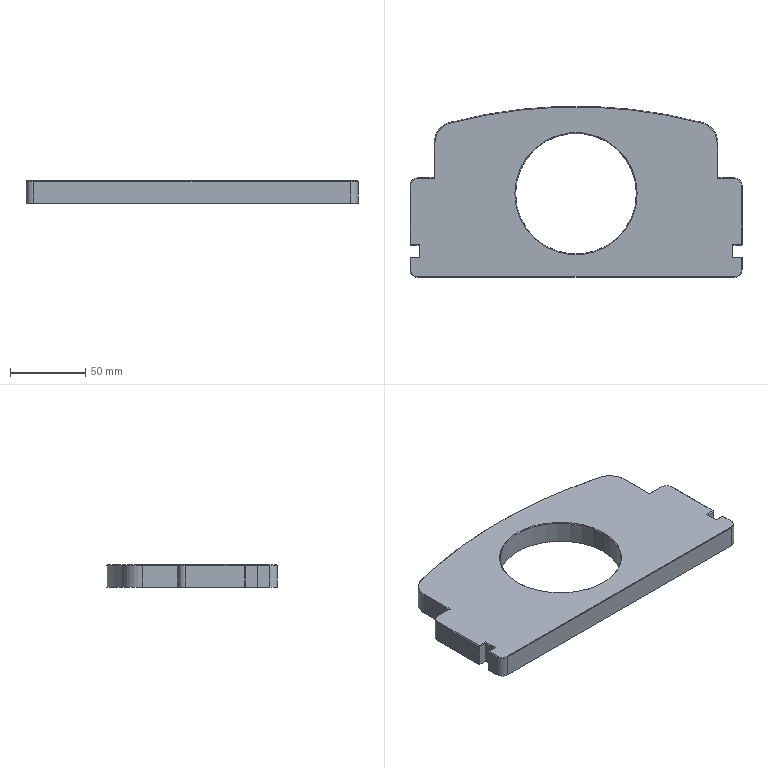Part | SolidWorks | features ICE 4, Chamfer 3, Extrusion 1, Fillet 1, HoleWzd 1 | 1 solid | 54 faces | box 220 x 113.5 x 15 mm | volume 261073 mm3 | plane 36 | cone 9 | cylinder 9 | commonest cylinder face diameters 10 x4 28 x2 80 x2 660 x1
STEP:
#1=CARTESIAN_POINT('',(-40.,55.5,7.));
#2=VERTEX_POINT('',#1);
#3=CARTESIAN_POINT('',(40.,55.5,7.));
#4=VERTEX_POINT('',#3);
#5=CARTESIAN_POINT('',(0.,55.5,7.));
#6=DIRECTION('',(0.,0.,1.));
#7=DIRECTION('',(1.,0.,0.));
#8=AXIS2_PLACEMENT_3D('',#5,#6,#7);
#9=CIRCLE('',#8,40.);
#10=EDGE_CURVE('',#2,#4,#9,.T.);
#11=ORIENTED_EDGE('',*,*,#10,.F.);
#12=CARTESIAN_POINT('',(-40.5,55.5,7.5));
#13=VERTEX_POINT('',#12);
#14=CARTESIAN_POINT('',(-40.,55.5,7.));
#15=DIRECTION('',(-0.7071,0.,0.7071));
#16=VECTOR('',#15,1000.);
#17=LINE('',#14,#16);
#18=EDGE_CURVE('',#2,#13,#17,.T.);
#19=ORIENTED_EDGE('',*,*,#18,.T.);
#20=CARTESIAN_POINT('',(40.5,55.5,7.5));
#21=VERTEX_POINT('',#20);
#22=CARTESIAN_POINT('',(0.,55.5,7.5));
#23=DIRECTION('',(0.,0.,-1.));
#24=DIRECTION('',(1.,0.,0.));
#25=AXIS2_PLACEMENT_3D('',#22,#23,#24);
#26=CIRCLE('',#25,40.5);
#27=EDGE_CURVE('',#21,#13,#26,.T.);
#28=ORIENTED_EDGE('',*,*,#27,.F.);
#29=CARTESIAN_POINT('',(40.,55.5,7.));
#30=DIRECTION('',(0.7071,0.,0.7071));
#31=VECTOR('',#30,1000.);
#32=LINE('',#29,#31);
#33=EDGE_CURVE('',#4,#21,#32,.T.);
#34=ORIENTED_EDGE('',*,*,#33,.F.);
#35=EDGE_LOOP('',(#11,#19,#28,#34));
#36=FACE_OUTER_BOUND('',#35,.T.);
#37=CARTESIAN_POINT('',(0.,55.5,7.));
#38=DIRECTION('',(0.,0.,1.));
#39=DIRECTION('',(1.,0.,0.));
#40=AXIS2_PLACEMENT_3D('',#37,#38,#39);
#41=CONICAL_SURFACE('',#40,40.,0.7854);
#42=ADVANCED_FACE('',(#36),#41,.F.);
#43=CARTESIAN_POINT('',(-40.,55.5,-7.5));
#44=VERTEX_POINT('',#43);
#45=CARTESIAN_POINT('',(40.,55.5,-7.5));
#46=VERTEX_POINT('',#45);
#47=CARTESIAN_POINT('',(0.,55.5,-7.5));
#48=DIRECTION('',(0.,0.,1.));
#49=DIRECTION('',(1.,0.,0.));
#50=AXIS2_PLACEMENT_3D('',#47,#48,#49);
#51=CIRCLE('',#50,40.);
#52=EDGE_CURVE('',#44,#46,#51,.T.);
#53=ORIENTED_EDGE('',*,*,#52,.F.);
#54=CARTESIAN_POINT('',(-40.,55.5,-7.5));
#55=DIRECTION('',(0.,0.,1.));
#56=VECTOR('',#55,1000.);
#57=LINE('',#54,#56);
#58=EDGE_CURVE('',#44,#2,#57,.T.);
#59=ORIENTED_EDGE('',*,*,#58,.T.);
#60=ORIENTED_EDGE('',*,*,#10,.T.);
#61=CARTESIAN_POINT('',(40.,55.5,-7.5));
#62=DIRECTION('',(0.,0.,1.));
#63=VECTOR('',#62,1000.);
#64=LINE('',#61,#63);
#65=EDGE_CURVE('',#46,#4,#64,.T.);
#66=ORIENTED_EDGE('',*,*,#65,.F.);
#67=EDGE_LOOP('',(#53,#59,#60,#66));
#68=FACE_OUTER_BOUND('',#67,.T.);
#69=CARTESIAN_POINT('',(0.,55.5,-7.5));
#70=DIRECTION('',(0.,0.,1.));
#71=DIRECTION('',(1.,0.,0.));
#72=AXIS2_PLACEMENT_3D('',#69,#70,#71);
#73=CYLINDRICAL_SURFACE('',#72,40.);
#74=ADVANCED_FACE('',(#68),#73,.F.);
#75=CARTESIAN_POINT('',(110.,5.,-7.5));
#76=VERTEX_POINT('',#75);
#77=CARTESIAN_POINT('',(110.,13.,-7.5));
#78=VERTEX_POINT('',#77);
#79=CARTESIAN_POINT('',(110.,121.,-7.5));
#80=DIRECTION('',(0.,1.,0.));
#81=VECTOR('',#80,1000.);
#82=LINE('',#79,#81);
#83=EDGE_CURVE('',#76,#78,#82,.T.);
#84=ORIENTED_EDGE('',*,*,#83,.T.);
#85=CARTESIAN_POINT('',(110.,13.,7.));
#86=VERTEX_POINT('',#85);
#87=CARTESIAN_POINT('',(110.,13.,7.5));
#88=DIRECTION('',(0.,0.,1.));
#89=VECTOR('',#88,1000.);
#90=LINE('',#87,#89);
#91=EDGE_CURVE('',#78,#86,#90,.T.);
#92=ORIENTED_EDGE('',*,*,#91,.T.);
#93=CARTESIAN_POINT('',(110.,5.,7.));
#94=VERTEX_POINT('',#93);
#95=CARTESIAN_POINT('',(110.,5.,7.));
#96=DIRECTION('',(0.,-1.,0.));
#97=VECTOR('',#96,1000.);
#98=LINE('',#95,#97);
#99=EDGE_CURVE('',#86,#94,#98,.T.);
#100=ORIENTED_EDGE('',*,*,#99,.T.);
#101=CARTESIAN_POINT('',(110.,5.,7.5));
#102=DIRECTION('',(0.,0.,-1.));
#103=VECTOR('',#102,1000.);
#104=LINE('',#101,#103);
#105=EDGE_CURVE('',#94,#76,#104,.T.);
#106=ORIENTED_EDGE('',*,*,#105,.T.);
#107=EDGE_LOOP('',(#84,#92,#100,#106));
#108=FACE_OUTER_BOUND('',#107,.T.);
#109=CARTESIAN_POINT('',(110.,121.,7.5));
#110=DIRECTION('',(-1.,0.,0.));
#111=DIRECTION('',(0.,-1.,0.));
#112=AXIS2_PLACEMENT_3D('',#109,#110,#111);
#113=PLANE('',#112);
#114=ADVANCED_FACE('',(#108),#113,.F.);
#115=CARTESIAN_POINT('',(-110.,61.,-7.5));
#116=VERTEX_POINT('',#115);
#117=CARTESIAN_POINT('',(-110.,22.,-7.5));
#118=VERTEX_POINT('',#117);
#119=CARTESIAN_POINT('',(-110.,121.,-7.5));
#120=DIRECTION('',(0.,-1.,0.));
#121=VECTOR('',#120,1000.);
#122=LINE('',#119,#121);
#123=EDGE_CURVE('',#116,#118,#122,.T.);
#124=ORIENTED_EDGE('',*,*,#123,.T.);
#125=CARTESIAN_POINT('',(-110.,22.,7.));
#126=VERTEX_POINT('',#125);
#127=CARTESIAN_POINT('',(-110.,22.,7.5));
#128=DIRECTION('',(0.,0.,1.));
#129=VECTOR('',#128,1000.);
#130=LINE('',#127,#129);
#131=EDGE_CURVE('',#118,#126,#130,.T.);
#132=ORIENTED_EDGE('',*,*,#131,.T.);
#133=CARTESIAN_POINT('',(-110.,61.,7.));
#134=VERTEX_POINT('',#133);
#135=CARTESIAN_POINT('',(-110.,61.,7.));
#136=DIRECTION('',(0.,1.,0.));
#137=VECTOR('',#136,1000.);
#138=LINE('',#135,#137);
#139=EDGE_CURVE('',#126,#134,#138,.T.);
#140=ORIENTED_EDGE('',*,*,#139,.T.);
#141=CARTESIAN_POINT('',(-110.,61.,7.5));
#142=DIRECTION('',(0.,0.,-1.));
#143=VECTOR('',#142,1000.);
#144=LINE('',#141,#143);
#145=EDGE_CURVE('',#134,#116,#144,.T.);
#146=ORIENTED_EDGE('',*,*,#145,.T.);
#147=EDGE_LOOP('',(#124,#132,#140,#146));
#148=FACE_OUTER_BOUND('',#147,.T.);
#149=CARTESIAN_POINT('',(-110.,121.,7.5));
#150=DIRECTION('',(1.,0.,0.));
#151=DIRECTION('',(0.,1.,0.));
#152=AXIS2_PLACEMENT_3D('',#149,#150,#151);
#153=PLANE('',#152);
#154=ADVANCED_FACE('',(#148),#153,.F.);
#155=CARTESIAN_POINT('',(-110.,5.,7.));
#156=VERTEX_POINT('',#155);
#157=CARTESIAN_POINT('',(-110.,13.,7.));
#158=VERTEX_POINT('',#157);
#159=CARTESIAN_POINT('',(-110.,13.5,7.));
#160=DIRECTION('',(0.,1.,0.));
#161=VECTOR('',#160,1000.);
#162=LINE('',#159,#161);
#163=EDGE_CURVE('',#156,#158,#162,.T.);
#164=ORIENTED_EDGE('',*,*,#163,.T.);
#165=CARTESIAN_POINT('',(-110.,13.,-7.5));
#166=VERTEX_POINT('',#165);
#167=CARTESIAN_POINT('',(-110.,13.,7.5));
#168=DIRECTION('',(0.,0.,-1.));
#169=VECTOR('',#168,1000.);
#170=LINE('',#167,#169);
#171=EDGE_CURVE('',#158,#166,#170,.T.);
#172=ORIENTED_EDGE('',*,*,#171,.T.);
#173=CARTESIAN_POINT('',(-110.,5.,-7.5));
#174=VERTEX_POINT('',#173);
#175=CARTESIAN_POINT('',(-110.,121.,-7.5));
#176=DIRECTION('',(0.,-1.,0.));
#177=VECTOR('',#176,1000.);
#178=LINE('',#175,#177);
#179=EDGE_CURVE('',#166,#174,#178,.T.);
#180=ORIENTED_EDGE('',*,*,#179,.T.);
#181=CARTESIAN_POINT('',(-110.,5.,7.5));
#182=DIRECTION('',(0.,0.,1.));
#183=VECTOR('',#182,1000.);
#184=LINE('',#181,#183);
#185=EDGE_CURVE('',#174,#156,#184,.T.);
#186=ORIENTED_EDGE('',*,*,#185,.T.);
#187=EDGE_LOOP('',(#164,#172,#180,#186));
#188=FACE_OUTER_BOUND('',#187,.T.);
#189=CARTESIAN_POINT('',(-110.,121.,7.5));
#190=DIRECTION('',(1.,0.,0.));
#191=DIRECTION('',(0.,1.,0.));
#192=AXIS2_PLACEMENT_3D('',#189,#190,#191);
#193=PLANE('',#192);
#194=ADVANCED_FACE('',(#188),#193,.F.);
#195=CARTESIAN_POINT('',(105.,0.,-7.5));
#196=VERTEX_POINT('',#195);
#197=CARTESIAN_POINT('',(105.,0.,7.));
#198=VERTEX_POINT('',#197);
#199=CARTESIAN_POINT('',(105.,0.,7.5));
#200=DIRECTION('',(0.,0.,1.));
#201=VECTOR('',#200,1000.);
#202=LINE('',#199,#201);
#203=EDGE_CURVE('',#196,#198,#202,.T.);
#204=ORIENTED_EDGE('',*,*,#203,.T.);
#205=CARTESIAN_POINT('',(-105.,0.,7.));
#206=VERTEX_POINT('',#205);
#207=CARTESIAN_POINT('',(-105.,0.,7.));
#208=DIRECTION('',(-1.,0.,0.));
#209=VECTOR('',#208,1000.);
#210=LINE('',#207,#209);
#211=EDGE_CURVE('',#198,#206,#210,.T.);
#212=ORIENTED_EDGE('',*,*,#211,.T.);
#213=CARTESIAN_POINT('',(-105.,0.,-7.5));
#214=VERTEX_POINT('',#213);
#215=CARTESIAN_POINT('',(-105.,0.,7.5));
#216=DIRECTION('',(0.,0.,-1.));
#217=VECTOR('',#216,1000.);
#218=LINE('',#215,#217);
#219=EDGE_CURVE('',#206,#214,#218,.T.);
#220=ORIENTED_EDGE('',*,*,#219,.T.);
#221=CARTESIAN_POINT('',(-110.,0.,-7.5));
#222=DIRECTION('',(1.,0.,0.));
#223=VECTOR('',#222,1000.);
#224=LINE('',#221,#223);
#225=EDGE_CURVE('',#214,#196,#224,.T.);
#226=ORIENTED_EDGE('',*,*,#225,.T.);
#227=EDGE_LOOP('',(#204,#212,#220,#226));
#228=FACE_OUTER_BOUND('',#227,.T.);
#229=CARTESIAN_POINT('',(-110.,0.,7.5));
#230=DIRECTION('',(0.,1.,0.));
#231=DIRECTION('',(0.,0.,1.));
#232=AXIS2_PLACEMENT_3D('',#229,#230,#231);
#233=PLANE('',#232);
#234=ADVANCED_FACE('',(#228),#233,.F.);
#235=CARTESIAN_POINT('',(110.,61.,7.));
#236=VERTEX_POINT('',#235);
#237=CARTESIAN_POINT('',(110.,22.,7.));
#238=VERTEX_POINT('',#237);
#239=CARTESIAN_POINT('',(110.,21.5,7.));
#240=DIRECTION('',(0.,-1.,0.));
#241=VECTOR('',#240,1000.);
#242=LINE('',#239,#241);
#243=EDGE_CURVE('',#236,#238,#242,.T.);
#244=ORIENTED_EDGE('',*,*,#243,.T.);
#245=CARTESIAN_POINT('',(110.,22.,-7.5));
#246=VERTEX_POINT('',#245);
#247=CARTESIAN_POINT('',(110.,22.,7.5));
#248=DIRECTION('',(0.,0.,-1.));
#249=VECTOR('',#248,1000.);
#250=LINE('',#247,#249);
#251=EDGE_CURVE('',#238,#246,#250,.T.);
#252=ORIENTED_EDGE('',*,*,#251,.T.);
#253=CARTESIAN_POINT('',(110.,61.,-7.5));
#254=VERTEX_POINT('',#253);
#255=CARTESIAN_POINT('',(110.,121.,-7.5));
#256=DIRECTION('',(0.,1.,0.));
#257=VECTOR('',#256,1000.);
#258=LINE('',#255,#257);
#259=EDGE_CURVE('',#246,#254,#258,.T.);
#260=ORIENTED_EDGE('',*,*,#259,.T.);
#261=CARTESIAN_POINT('',(110.,61.,7.5));
#262=DIRECTION('',(0.,0.,1.));
#263=VECTOR('',#262,1000.);
#264=LINE('',#261,#263);
#265=EDGE_CURVE('',#254,#236,#264,.T.);
#266=ORIENTED_EDGE('',*,*,#265,.T.);
#267=EDGE_LOOP('',(#244,#252,#260,#266));
#268=FACE_OUTER_BOUND('',#267,.T.);
#269=CARTESIAN_POINT('',(110.,121.,7.5));
#270=DIRECTION('',(-1.,0.,0.));
#271=DIRECTION('',(0.,-1.,0.));
#272=AXIS2_PLACEMENT_3D('',#269,#270,#271);
#273=PLANE('',#272);
#274=ADVANCED_FACE('',(#268),#273,.F.);
#275=ORIENTED_EDGE('',*,*,#27,.T.);
#276=CARTESIAN_POINT('',(0.,55.5,7.5));
#277=DIRECTION('',(0.,0.,-1.));
#278=DIRECTION('',(1.,0.,0.));
#279=AXIS2_PLACEMENT_3D('',#276,#277,#278);
#280=CIRCLE('',#279,40.5);
#281=EDGE_CURVE('',#13,#21,#280,.T.);
#282=ORIENTED_EDGE('',*,*,#281,.T.);
#283=EDGE_LOOP('',(#275,#282));
#284=FACE_BOUND('',#283,.T.);
#285=CARTESIAN_POINT('',(-109.5,13.,7.5));
#286=VERTEX_POINT('',#285);
#287=CARTESIAN_POINT('',(-109.5,5.,7.5));
#288=VERTEX_POINT('',#287);
#289=CARTESIAN_POINT('',(-109.5,5.,7.5));
#290=DIRECTION('',(0.,-1.,0.));
#291=VECTOR('',#290,1000.);
#292=LINE('',#289,#291);
#293=EDGE_CURVE('',#286,#288,#292,.T.);
#294=ORIENTED_EDGE('',*,*,#293,.T.);
#295=CARTESIAN_POINT('',(-105.,0.5,7.5));
#296=VERTEX_POINT('',#295);
#297=CARTESIAN_POINT('',(-105.,5.,7.5));
#298=DIRECTION('',(0.,0.,1.));
#299=DIRECTION('',(1.,0.,0.));
#300=AXIS2_PLACEMENT_3D('',#297,#298,#299);
#301=CIRCLE('',#300,4.5);
#302=EDGE_CURVE('',#288,#296,#301,.T.);
#303=ORIENTED_EDGE('',*,*,#302,.T.);
#304=CARTESIAN_POINT('',(105.,0.5,7.5));
#305=VERTEX_POINT('',#304);
#306=CARTESIAN_POINT('',(105.,0.5,7.5));
#307=DIRECTION('',(1.,0.,0.));
#308=VECTOR('',#307,1000.);
#309=LINE('',#306,#308);
#310=EDGE_CURVE('',#296,#305,#309,.T.);
#311=ORIENTED_EDGE('',*,*,#310,.T.);
#312=CARTESIAN_POINT('',(109.5,5.,7.5));
#313=VERTEX_POINT('',#312);
#314=CARTESIAN_POINT('',(105.,5.,7.5));
#315=DIRECTION('',(0.,0.,1.));
#316=DIRECTION('',(1.,0.,0.));
#317=AXIS2_PLACEMENT_3D('',#314,#315,#316);
#318=CIRCLE('',#317,4.5);
#319=EDGE_CURVE('',#305,#313,#318,.T.);
#320=ORIENTED_EDGE('',*,*,#319,.T.);
#321=CARTESIAN_POINT('',(109.5,13.,7.5));
#322=VERTEX_POINT('',#321);
#323=CARTESIAN_POINT('',(109.5,13.5,7.5));
#324=DIRECTION('',(0.,1.,0.));
#325=VECTOR('',#324,1000.);
#326=LINE('',#323,#325);
#327=EDGE_CURVE('',#313,#322,#326,.T.);
#328=ORIENTED_EDGE('',*,*,#327,.T.);
#329=CARTESIAN_POINT('',(103.5,13.,7.5));
#330=VERTEX_POINT('',#329);
#331=CARTESIAN_POINT('',(104.,13.,7.5));
#332=DIRECTION('',(-1.,0.,0.));
#333=VECTOR('',#332,1000.);
#334=LINE('',#331,#333);
#335=EDGE_CURVE('',#322,#330,#334,.T.);
#336=ORIENTED_EDGE('',*,*,#335,.T.);
#337=CARTESIAN_POINT('',(103.5,22.,7.5));
#338=VERTEX_POINT('',#337);
#339=CARTESIAN_POINT('',(103.5,21.5,7.5));
#340=DIRECTION('',(0.,1.,0.));
#341=VECTOR('',#340,1000.);
#342=LINE('',#339,#341);
#343=EDGE_CURVE('',#330,#338,#342,.T.);
#344=ORIENTED_EDGE('',*,*,#343,.T.);
#345=CARTESIAN_POINT('',(109.5,22.,7.5));
#346=VERTEX_POINT('',#345);
#347=CARTESIAN_POINT('',(110.,22.,7.5));
#348=DIRECTION('',(1.,0.,0.));
#349=VECTOR('',#348,1000.);
#350=LINE('',#347,#349);
#351=EDGE_CURVE('',#338,#346,#350,.T.);
#352=ORIENTED_EDGE('',*,*,#351,.T.);
#353=CARTESIAN_POINT('',(109.5,61.,7.5));
#354=VERTEX_POINT('',#353);
#355=CARTESIAN_POINT('',(109.5,61.,7.5));
#356=DIRECTION('',(0.,1.,0.));
#357=VECTOR('',#356,1000.);
#358=LINE('',#355,#357);
#359=EDGE_CURVE('',#346,#354,#358,.T.);
#360=ORIENTED_EDGE('',*,*,#359,.T.);
#361=CARTESIAN_POINT('',(105.,65.5,7.5));
#362=VERTEX_POINT('',#361);
#363=CARTESIAN_POINT('',(105.,61.,7.5));
#364=DIRECTION('',(0.,0.,1.));
#365=DIRECTION('',(1.,0.,0.));
#366=AXIS2_PLACEMENT_3D('',#363,#364,#365);
#367=CIRCLE('',#366,4.5);
#368=EDGE_CURVE('',#354,#362,#367,.T.);
#369=ORIENTED_EDGE('',*,*,#368,.T.);
#370=CARTESIAN_POINT('',(93.5,65.5,7.5));
#371=VERTEX_POINT('',#370);
#372=CARTESIAN_POINT('',(94.,65.5,7.5));
#373=DIRECTION('',(-1.,0.,0.));
#374=VECTOR('',#373,1000.);
#375=LINE('',#372,#374);
#376=EDGE_CURVE('',#362,#371,#375,.T.);
#377=ORIENTED_EDGE('',*,*,#376,.T.);
#378=CARTESIAN_POINT('',(93.5,89.206,7.5));
#379=VERTEX_POINT('',#378);
#380=CARTESIAN_POINT('',(93.5,89.206,7.5));
#381=DIRECTION('',(0.,1.,0.));
#382=VECTOR('',#381,1000.);
#383=LINE('',#380,#382);
#384=EDGE_CURVE('',#371,#379,#383,.T.);
#385=ORIENTED_EDGE('',*,*,#384,.T.);
#386=CARTESIAN_POINT('',(83.418,102.266,7.5));
#387=VERTEX_POINT('',#386);
#388=CARTESIAN_POINT('',(80.,89.206,7.5));
#389=DIRECTION('',(0.,0.,1.));
#390=DIRECTION('',(1.,0.,0.));
#391=AXIS2_PLACEMENT_3D('',#388,#389,#390);
#392=CIRCLE('',#391,13.5);
#393=EDGE_CURVE('',#379,#387,#392,.T.);
#394=ORIENTED_EDGE('',*,*,#393,.T.);
#395=CARTESIAN_POINT('',(-83.418,102.266,7.5));
#396=VERTEX_POINT('',#395);
#397=CARTESIAN_POINT('',(0.,-216.5,7.5));
#398=DIRECTION('',(0.,0.,1.));
#399=DIRECTION('',(1.,0.,0.));
#400=AXIS2_PLACEMENT_3D('',#397,#398,#399);
#401=CIRCLE('',#400,329.5);
#402=EDGE_CURVE('',#387,#396,#401,.T.);
#403=ORIENTED_EDGE('',*,*,#402,.T.);
#404=CARTESIAN_POINT('',(-93.5,89.206,7.5));
#405=VERTEX_POINT('',#404);
#406=CARTESIAN_POINT('',(-80.,89.206,7.5));
#407=DIRECTION('',(0.,0.,1.));
#408=DIRECTION('',(1.,0.,0.));
#409=AXIS2_PLACEMENT_3D('',#406,#407,#408);
#410=CIRCLE('',#409,13.5);
#411=EDGE_CURVE('',#396,#405,#410,.T.);
#412=ORIENTED_EDGE('',*,*,#411,.T.);
#413=CARTESIAN_POINT('',(-93.5,65.5,7.5));
#414=VERTEX_POINT('',#413);
#415=CARTESIAN_POINT('',(-93.5,66.,7.5));
#416=DIRECTION('',(0.,-1.,0.));
#417=VECTOR('',#416,1000.);
#418=LINE('',#415,#417);
#419=EDGE_CURVE('',#405,#414,#418,.T.);
#420=ORIENTED_EDGE('',*,*,#419,.T.);
#421=CARTESIAN_POINT('',(-105.,65.5,7.5));
#422=VERTEX_POINT('',#421);
#423=CARTESIAN_POINT('',(-105.,65.5,7.5));
#424=DIRECTION('',(-1.,0.,0.));
#425=VECTOR('',#424,1000.);
#426=LINE('',#423,#425);
#427=EDGE_CURVE('',#414,#422,#426,.T.);
#428=ORIENTED_EDGE('',*,*,#427,.T.);
#429=CARTESIAN_POINT('',(-109.5,61.,7.5));
#430=VERTEX_POINT('',#429);
#431=CARTESIAN_POINT('',(-105.,61.,7.5));
#432=DIRECTION('',(0.,0.,1.));
#433=DIRECTION('',(1.,0.,0.));
#434=AXIS2_PLACEMENT_3D('',#431,#432,#433);
#435=CIRCLE('',#434,4.5);
#436=EDGE_CURVE('',#422,#430,#435,.T.);
#437=ORIENTED_EDGE('',*,*,#436,.T.);
#438=CARTESIAN_POINT('',(-109.5,22.,7.5));
#439=VERTEX_POINT('',#438);
#440=CARTESIAN_POINT('',(-109.5,21.5,7.5));
#441=DIRECTION('',(0.,-1.,0.));
#442=VECTOR('',#441,1000.);
#443=LINE('',#440,#442);
#444=EDGE_CURVE('',#430,#439,#443,.T.);
#445=ORIENTED_EDGE('',*,*,#444,.T.);
#446=CARTESIAN_POINT('',(-103.5,22.,7.5));
#447=VERTEX_POINT('',#446);
#448=CARTESIAN_POINT('',(-104.,22.,7.5));
#449=DIRECTION('',(1.,0.,0.));
#450=VECTOR('',#449,1000.);
#451=LINE('',#448,#450);
#452=EDGE_CURVE('',#439,#447,#451,.T.);
#453=ORIENTED_EDGE('',*,*,#452,.T.);
#454=CARTESIAN_POINT('',(-103.5,13.,7.5));
#455=VERTEX_POINT('',#454);
#456=CARTESIAN_POINT('',(-103.5,13.5,7.5));
#457=DIRECTION('',(0.,-1.,0.));
#458=VECTOR('',#457,1000.);
#459=LINE('',#456,#458);
#460=EDGE_CURVE('',#447,#455,#459,.T.);
#461=ORIENTED_EDGE('',*,*,#460,.T.);
#462=CARTESIAN_POINT('',(-110.,13.,7.5));
#463=DIRECTION('',(-1.,0.,0.));
#464=VECTOR('',#463,1000.);
#465=LINE('',#462,#464);
#466=EDGE_CURVE('',#455,#286,#465,.T.);
#467=ORIENTED_EDGE('',*,*,#466,.T.);
#468=EDGE_LOOP('',(#294,#303,#311,#320,#328,#336,#344,#352,#360,#369,#377,#385,#394,#403,#412,#420,#428,#437,#445,#453,#461,#467));
#469=FACE_OUTER_BOUND('',#468,.T.);
#470=CARTESIAN_POINT('',(0.,0.,7.5));
#471=DIRECTION('',(0.,0.,1.));
#472=DIRECTION('',(1.,0.,0.));
#473=AXIS2_PLACEMENT_3D('',#470,#471,#472);
#474=PLANE('',#473);
#475=ADVANCED_FACE('',(#284,#469),#474,.T.);
#476=CARTESIAN_POINT('',(0.,55.5,-7.5));
#477=DIRECTION('',(0.,0.,1.));
#478=DIRECTION('',(1.,0.,0.));
#479=AXIS2_PLACEMENT_3D('',#476,#477,#478);
#480=CIRCLE('',#479,40.);
#481=EDGE_CURVE('',#46,#44,#480,.T.);
#482=ORIENTED_EDGE('',*,*,#481,.T.);
#483=ORIENTED_EDGE('',*,*,#52,.T.);
#484=EDGE_LOOP('',(#482,#483));
#485=FACE_BOUND('',#484,.T.);
#486=CARTESIAN_POINT('',(104.,13.5,-7.5));
#487=VERTEX_POINT('',#486);
#488=CARTESIAN_POINT('',(109.5,13.5,-7.5));
#489=VERTEX_POINT('',#488);
#490=CARTESIAN_POINT('',(110.,13.5,-7.5));
#491=DIRECTION('',(1.,0.,0.));
#492=VECTOR('',#491,1000.);
#493=LINE('',#490,#492);
#494=EDGE_CURVE('',#487,#489,#493,.T.);
#495=ORIENTED_EDGE('',*,*,#494,.T.);
#496=CARTESIAN_POINT('',(110.,13.,-7.5));
#497=DIRECTION('',(0.7071,-0.7071,0.));
#498=VECTOR('',#497,1000.);
#499=LINE('',#496,#498);
#500=EDGE_CURVE('',#489,#78,#499,.T.);
#501=ORIENTED_EDGE('',*,*,#500,.T.);
#502=ORIENTED_EDGE('',*,*,#83,.F.);
#503=CARTESIAN_POINT('',(105.,5.,-7.5));
#504=DIRECTION('',(0.,0.,-1.));
#505=DIRECTION('',(1.,0.,0.));
#506=AXIS2_PLACEMENT_3D('',#503,#504,#505);
#507=CIRCLE('',#506,5.);
#508=EDGE_CURVE('',#76,#196,#507,.T.);
#509=ORIENTED_EDGE('',*,*,#508,.T.);
#510=ORIENTED_EDGE('',*,*,#225,.F.);
#511=CARTESIAN_POINT('',(-105.,5.,-7.5));
#512=DIRECTION('',(0.,0.,-1.));
#513=DIRECTION('',(1.,0.,0.));
#514=AXIS2_PLACEMENT_3D('',#511,#512,#513);
#515=CIRCLE('',#514,5.);
#516=EDGE_CURVE('',#214,#174,#515,.T.);
#517=ORIENTED_EDGE('',*,*,#516,.T.);
#518=ORIENTED_EDGE('',*,*,#179,.F.);
#519=CARTESIAN_POINT('',(-109.5,13.5,-7.5));
#520=VERTEX_POINT('',#519);
#521=CARTESIAN_POINT('',(-109.5,13.5,-7.5));
#522=DIRECTION('',(0.7071,0.7071,0.));
#523=VECTOR('',#522,1000.);
#524=LINE('',#521,#523);
#525=EDGE_CURVE('',#166,#520,#524,.T.);
#526=ORIENTED_EDGE('',*,*,#525,.T.);
#527=CARTESIAN_POINT('',(-104.,13.5,-7.5));
#528=VERTEX_POINT('',#527);
#529=CARTESIAN_POINT('',(-110.,13.5,-7.5));
#530=DIRECTION('',(1.,0.,0.));
#531=VECTOR('',#530,1000.);
#532=LINE('',#529,#531);
#533=EDGE_CURVE('',#520,#528,#532,.T.);
#534=ORIENTED_EDGE('',*,*,#533,.T.);
#535=CARTESIAN_POINT('',(-104.,21.5,-7.5));
#536=VERTEX_POINT('',#535);
#537=CARTESIAN_POINT('',(-104.,21.5,-7.5));
#538=DIRECTION('',(0.,1.,0.));
#539=VECTOR('',#538,1000.);
#540=LINE('',#537,#539);
#541=EDGE_CURVE('',#528,#536,#540,.T.);
#542=ORIENTED_EDGE('',*,*,#541,.T.);
#543=CARTESIAN_POINT('',(-109.5,21.5,-7.5));
#544=VERTEX_POINT('',#543);
#545=CARTESIAN_POINT('',(-110.,21.5,-7.5));
#546=DIRECTION('',(-1.,0.,0.));
#547=VECTOR('',#546,1000.);
#548=LINE('',#545,#547);
#549=EDGE_CURVE('',#536,#544,#548,.T.);
#550=ORIENTED_EDGE('',*,*,#549,.T.);
#551=CARTESIAN_POINT('',(-110.,22.,-7.5));
#552=DIRECTION('',(-0.7071,0.7071,0.));
#553=VECTOR('',#552,1000.);
#554=LINE('',#551,#553);
#555=EDGE_CURVE('',#544,#118,#554,.T.);
#556=ORIENTED_EDGE('',*,*,#555,.T.);
#557=ORIENTED_EDGE('',*,*,#123,.F.);
#558=CARTESIAN_POINT('',(-105.,66.,-7.5));
#559=VERTEX_POINT('',#558);
#560=CARTESIAN_POINT('',(-105.,61.,-7.5));
#561=DIRECTION('',(0.,0.,-1.));
#562=DIRECTION('',(1.,0.,0.));
#563=AXIS2_PLACEMENT_3D('',#560,#561,#562);
#564=CIRCLE('',#563,5.);
#565=EDGE_CURVE('',#116,#559,#564,.T.);
#566=ORIENTED_EDGE('',*,*,#565,.T.);
#567=CARTESIAN_POINT('',(-94.,66.,-7.5));
#568=VERTEX_POINT('',#567);
#569=CARTESIAN_POINT('',(-94.,66.,-7.5));
#570=DIRECTION('',(1.,0.,0.));
#571=VECTOR('',#570,1000.);
#572=LINE('',#569,#571);
#573=EDGE_CURVE('',#559,#568,#572,.T.);
#574=ORIENTED_EDGE('',*,*,#573,.T.);
#575=CARTESIAN_POINT('',(-94.,89.206,-7.5));
#576=VERTEX_POINT('',#575);
#577=CARTESIAN_POINT('',(-94.,66.,-7.5));
#578=DIRECTION('',(0.,1.,0.));
#579=VECTOR('',#578,1000.);
#580=LINE('',#577,#579);
#581=EDGE_CURVE('',#568,#576,#580,.T.);
#582=ORIENTED_EDGE('',*,*,#581,.T.);
#583=CARTESIAN_POINT('',(-83.544,102.75,-7.5));
#584=VERTEX_POINT('',#583);
#585=CARTESIAN_POINT('',(-80.,89.206,-7.5));
#586=DIRECTION('',(0.,0.,-1.));
#587=DIRECTION('',(1.,0.,0.));
#588=AXIS2_PLACEMENT_3D('',#585,#586,#587);
#589=CIRCLE('',#588,14.);
#590=EDGE_CURVE('',#576,#584,#589,.T.);
#591=ORIENTED_EDGE('',*,*,#590,.T.);
#592=CARTESIAN_POINT('',(83.544,102.75,-7.5));
#593=VERTEX_POINT('',#592);
#594=CARTESIAN_POINT('',(0.,-216.5,-7.5));
#595=DIRECTION('',(0.,0.,-1.));
#596=DIRECTION('',(1.,0.,0.));
#597=AXIS2_PLACEMENT_3D('',#594,#595,#596);
#598=CIRCLE('',#597,330.);
#599=EDGE_CURVE('',#584,#593,#598,.T.);
#600=ORIENTED_EDGE('',*,*,#599,.T.);
#601=CARTESIAN_POINT('',(94.,89.206,-7.5));
#602=VERTEX_POINT('',#601);
#603=CARTESIAN_POINT('',(80.,89.206,-7.5));
#604=DIRECTION('',(0.,0.,-1.));
#605=DIRECTION('',(-1.,0.,0.));
#606=AXIS2_PLACEMENT_3D('',#603,#604,#605);
#607=CIRCLE('',#606,14.);
#608=EDGE_CURVE('',#593,#602,#607,.T.);
#609=ORIENTED_EDGE('',*,*,#608,.T.);
#610=CARTESIAN_POINT('',(94.,66.,-7.5));
#611=VERTEX_POINT('',#610);
#612=CARTESIAN_POINT('',(94.,66.,-7.5));
#613=DIRECTION('',(0.,-1.,0.));
#614=VECTOR('',#613,1000.);
#615=LINE('',#612,#614);
#616=EDGE_CURVE('',#602,#611,#615,.T.);
#617=ORIENTED_EDGE('',*,*,#616,.T.);
#618=CARTESIAN_POINT('',(105.,66.,-7.5));
#619=VERTEX_POINT('',#618);
#620=CARTESIAN_POINT('',(110.,66.,-7.5));
#621=DIRECTION('',(1.,0.,0.));
#622=VECTOR('',#621,1000.);
#623=LINE('',#620,#622);
#624=EDGE_CURVE('',#611,#619,#623,.T.);
#625=ORIENTED_EDGE('',*,*,#624,.T.);
#626=CARTESIAN_POINT('',(105.,61.,-7.5));
#627=DIRECTION('',(0.,0.,-1.));
#628=DIRECTION('',(1.,0.,0.));
#629=AXIS2_PLACEMENT_3D('',#626,#627,#628);
#630=CIRCLE('',#629,5.);
#631=EDGE_CURVE('',#619,#254,#630,.T.);
#632=ORIENTED_EDGE('',*,*,#631,.T.);
#633=ORIENTED_EDGE('',*,*,#259,.F.);
#634=CARTESIAN_POINT('',(109.5,21.5,-7.5));
#635=VERTEX_POINT('',#634);
#636=CARTESIAN_POINT('',(109.5,21.5,-7.5));
#637=DIRECTION('',(-0.7071,-0.7071,0.));
#638=VECTOR('',#637,1000.);
#639=LINE('',#636,#638);
#640=EDGE_CURVE('',#246,#635,#639,.T.);
#641=ORIENTED_EDGE('',*,*,#640,.T.);
#642=CARTESIAN_POINT('',(104.,21.5,-7.5));
#643=VERTEX_POINT('',#642);
#644=CARTESIAN_POINT('',(110.,21.5,-7.5));
#645=DIRECTION('',(-1.,0.,0.));
#646=VECTOR('',#645,1000.);
#647=LINE('',#644,#646);
#648=EDGE_CURVE('',#635,#643,#647,.T.);
#649=ORIENTED_EDGE('',*,*,#648,.T.);
#650=CARTESIAN_POINT('',(104.,21.5,-7.5));
#651=DIRECTION('',(0.,-1.,0.));
#652=VECTOR('',#651,1000.);
#653=LINE('',#650,#652);
#654=EDGE_CURVE('',#643,#487,#653,.T.);
#655=ORIENTED_EDGE('',*,*,#654,.T.);
#656=EDGE_LOOP('',(#495,#501,#502,#509,#510,#517,#518,#526,#534,#542,#550,#556,#557,#566,#574,#582,#591,#600,#609,#617,#625,#632,#633,#641,#649,#655));
#657=FACE_OUTER_BOUND('',#656,.T.);
#658=CARTESIAN_POINT('',(0.,0.,-7.5));
#659=DIRECTION('',(0.,0.,1.));
#660=DIRECTION('',(1.,0.,0.));
#661=AXIS2_PLACEMENT_3D('',#658,#659,#660);
#662=PLANE('',#661);
#663=ADVANCED_FACE('',(#485,#657),#662,.F.);
#664=CARTESIAN_POINT('',(-104.,21.5,7.));
#665=VERTEX_POINT('',#664);
#666=CARTESIAN_POINT('',(-109.5,21.5,7.));
#667=VERTEX_POINT('',#666);
#668=CARTESIAN_POINT('',(-110.,21.5,7.));
#669=DIRECTION('',(-1.,0.,0.));
#670=VECTOR('',#669,1000.);
#671=LINE('',#668,#670);
#672=EDGE_CURVE('',#665,#667,#671,.T.);
#673=ORIENTED_EDGE('',*,*,#672,.T.);
#674=CARTESIAN_POINT('',(-109.5,21.5,-7.5));
#675=DIRECTION('',(0.,0.,-1.));
#676=VECTOR('',#675,1000.);
#677=LINE('',#674,#676);
#678=EDGE_CURVE('',#667,#544,#677,.T.);
#679=ORIENTED_EDGE('',*,*,#678,.T.);
#680=ORIENTED_EDGE('',*,*,#549,.F.);
#681=CARTESIAN_POINT('',(-104.,21.5,-7.5));
#682=DIRECTION('',(0.,0.,1.));
#683=VECTOR('',#682,1000.);
#684=LINE('',#681,#683);
#685=EDGE_CURVE('',#536,#665,#684,.T.);
#686=ORIENTED_EDGE('',*,*,#685,.T.);
#687=EDGE_LOOP('',(#673,#679,#680,#686));
#688=FACE_OUTER_BOUND('',#687,.T.);
#689=CARTESIAN_POINT('',(-110.,21.5,-7.5));
#690=DIRECTION('',(0.,1.,0.));
#691=DIRECTION('',(-1.,0.,0.));
#692=AXIS2_PLACEMENT_3D('',#689,#690,#691);
#693=PLANE('',#692);
#694=ADVANCED_FACE('',(#688),#693,.F.);
#695=CARTESIAN_POINT('',(-104.,13.5,7.));
#696=VERTEX_POINT('',#695);
#697=CARTESIAN_POINT('',(-104.,13.5,-7.5));
#698=DIRECTION('',(0.,0.,1.));
#699=VECTOR('',#698,1000.);
#700=LINE('',#697,#699);
#701=EDGE_CURVE('',#528,#696,#700,.T.);
#702=ORIENTED_EDGE('',*,*,#701,.T.);
#703=CARTESIAN_POINT('',(-104.,21.5,7.));
#704=DIRECTION('',(0.,1.,0.));
#705=VECTOR('',#704,1000.);
#706=LINE('',#703,#705);
#707=EDGE_CURVE('',#696,#665,#706,.T.);
#708=ORIENTED_EDGE('',*,*,#707,.T.);
#709=ORIENTED_EDGE('',*,*,#685,.F.);
#710=ORIENTED_EDGE('',*,*,#541,.F.);
#711=EDGE_LOOP('',(#702,#708,#709,#710));
#712=FACE_OUTER_BOUND('',#711,.T.);
#713=CARTESIAN_POINT('',(-104.,21.5,-7.5));
#714=DIRECTION('',(1.,0.,0.));
#715=DIRECTION('',(0.,0.,-1.));
#716=AXIS2_PLACEMENT_3D('',#713,#714,#715);
#717=PLANE('',#716);
#718=ADVANCED_FACE('',(#712),#717,.F.);
#719=ORIENTED_EDGE('',*,*,#533,.F.);
#720=CARTESIAN_POINT('',(-109.5,13.5,7.));
#721=VERTEX_POINT('',#720);
#722=CARTESIAN_POINT('',(-109.5,13.5,-7.5));
#723=DIRECTION('',(0.,0.,1.));
#724=VECTOR('',#723,1000.);
#725=LINE('',#722,#724);
#726=EDGE_CURVE('',#520,#721,#725,.T.);
#727=ORIENTED_EDGE('',*,*,#726,.T.);
#728=CARTESIAN_POINT('',(-104.,13.5,7.));
#729=DIRECTION('',(1.,0.,0.));
#730=VECTOR('',#729,1000.);
#731=LINE('',#728,#730);
#732=EDGE_CURVE('',#721,#696,#731,.T.);
#733=ORIENTED_EDGE('',*,*,#732,.T.);
#734=ORIENTED_EDGE('',*,*,#701,.F.);
#735=EDGE_LOOP('',(#719,#727,#733,#734));
#736=FACE_OUTER_BOUND('',#735,.T.);
#737=CARTESIAN_POINT('',(-110.,13.5,-7.5));
#738=DIRECTION('',(0.,-1.,0.));
#739=DIRECTION('',(0.,0.,-1.));
#740=AXIS2_PLACEMENT_3D('',#737,#738,#739);
#741=PLANE('',#740);
#742=ADVANCED_FACE('',(#736),#741,.F.);
#743=CARTESIAN_POINT('',(104.,13.5,7.));
#744=VERTEX_POINT('',#743);
#745=CARTESIAN_POINT('',(109.5,13.5,7.));
#746=VERTEX_POINT('',#745);
#747=CARTESIAN_POINT('',(110.,13.5,7.));
#748=DIRECTION('',(1.,0.,0.));
#749=VECTOR('',#748,1000.);
#750=LINE('',#747,#749);
#751=EDGE_CURVE('',#744,#746,#750,.T.);
#752=ORIENTED_EDGE('',*,*,#751,.T.);
#753=CARTESIAN_POINT('',(109.5,13.5,-7.5));
#754=DIRECTION('',(0.,0.,-1.));
#755=VECTOR('',#754,1000.);
#756=LINE('',#753,#755);
#757=EDGE_CURVE('',#746,#489,#756,.T.);
#758=ORIENTED_EDGE('',*,*,#757,.T.);
#759=ORIENTED_EDGE('',*,*,#494,.F.);
#760=CARTESIAN_POINT('',(104.,13.5,-7.5));
#761=DIRECTION('',(0.,0.,1.));
#762=VECTOR('',#761,1000.);
#763=LINE('',#760,#762);
#764=EDGE_CURVE('',#487,#744,#763,.T.);
#765=ORIENTED_EDGE('',*,*,#764,.T.);
#766=EDGE_LOOP('',(#752,#758,#759,#765));
#767=FACE_OUTER_BOUND('',#766,.T.);
#768=CARTESIAN_POINT('',(110.,13.5,-7.5));
#769=DIRECTION('',(0.,-1.,0.));
#770=DIRECTION('',(1.,0.,0.));
#771=AXIS2_PLACEMENT_3D('',#768,#769,#770);
#772=PLANE('',#771);
#773=ADVANCED_FACE('',(#767),#772,.F.);
#774=CARTESIAN_POINT('',(104.,21.5,7.));
#775=VERTEX_POINT('',#774);
#776=CARTESIAN_POINT('',(104.,21.5,-7.5));
#777=DIRECTION('',(0.,0.,1.));
#778=VECTOR('',#777,1000.);
#779=LINE('',#776,#778);
#780=EDGE_CURVE('',#643,#775,#779,.T.);
#781=ORIENTED_EDGE('',*,*,#780,.T.);
#782=CARTESIAN_POINT('',(104.,13.5,7.));
#783=DIRECTION('',(0.,-1.,0.));
#784=VECTOR('',#783,1000.);
#785=LINE('',#782,#784);
#786=EDGE_CURVE('',#775,#744,#785,.T.);
#787=ORIENTED_EDGE('',*,*,#786,.T.);
#788=ORIENTED_EDGE('',*,*,#764,.F.);
#789=ORIENTED_EDGE('',*,*,#654,.F.);
#790=EDGE_LOOP('',(#781,#787,#788,#789));
#791=FACE_OUTER_BOUND('',#790,.T.);
#792=CARTESIAN_POINT('',(104.,21.5,-7.5));
#793=DIRECTION('',(-1.,0.,0.));
#794=DIRECTION('',(0.,0.,1.));
#795=AXIS2_PLACEMENT_3D('',#792,#793,#794);
#796=PLANE('',#795);
#797=ADVANCED_FACE('',(#791),#796,.F.);
#798=ORIENTED_EDGE('',*,*,#648,.F.);
#799=CARTESIAN_POINT('',(109.5,21.5,7.));
#800=VERTEX_POINT('',#799);
#801=CARTESIAN_POINT('',(109.5,21.5,-7.5));
#802=DIRECTION('',(0.,0.,1.));
#803=VECTOR('',#802,1000.);
#804=LINE('',#801,#803);
#805=EDGE_CURVE('',#635,#800,#804,.T.);
#806=ORIENTED_EDGE('',*,*,#805,.T.);
#807=CARTESIAN_POINT('',(104.,21.5,7.));
#808=DIRECTION('',(-1.,0.,0.));
#809=VECTOR('',#808,1000.);
#810=LINE('',#807,#809);
#811=EDGE_CURVE('',#800,#775,#810,.T.);
#812=ORIENTED_EDGE('',*,*,#811,.T.);
#813=ORIENTED_EDGE('',*,*,#780,.F.);
#814=EDGE_LOOP('',(#798,#806,#812,#813));
#815=FACE_OUTER_BOUND('',#814,.T.);
#816=CARTESIAN_POINT('',(110.,21.5,-7.5));
#817=DIRECTION('',(0.,1.,0.));
#818=DIRECTION('',(-1.,0.,0.));
#819=AXIS2_PLACEMENT_3D('',#816,#817,#818);
#820=PLANE('',#819);
#821=ADVANCED_FACE('',(#815),#820,.F.);
#822=CARTESIAN_POINT('',(-94.,66.,7.));
#823=VERTEX_POINT('',#822);
#824=CARTESIAN_POINT('',(-94.,66.,-7.5));
#825=DIRECTION('',(0.,0.,1.));
#826=VECTOR('',#825,1000.);
#827=LINE('',#824,#826);
#828=EDGE_CURVE('',#568,#823,#827,.T.);
#829=ORIENTED_EDGE('',*,*,#828,.T.);
#830=CARTESIAN_POINT('',(-94.,89.206,7.));
#831=VERTEX_POINT('',#830);
#832=CARTESIAN_POINT('',(-94.,89.206,7.));
#833=DIRECTION('',(0.,1.,0.));
#834=VECTOR('',#833,1000.);
#835=LINE('',#832,#834);
#836=EDGE_CURVE('',#823,#831,#835,.T.);
#837=ORIENTED_EDGE('',*,*,#836,.T.);
#838=CARTESIAN_POINT('',(-94.,89.206,-7.5));
#839=DIRECTION('',(0.,0.,1.));
#840=VECTOR('',#839,1000.);
#841=LINE('',#838,#840);
#842=EDGE_CURVE('',#576,#831,#841,.T.);
#843=ORIENTED_EDGE('',*,*,#842,.F.);
#844=ORIENTED_EDGE('',*,*,#581,.F.);
#845=EDGE_LOOP('',(#829,#837,#843,#844));
#846=FACE_OUTER_BOUND('',#845,.T.);
#847=CARTESIAN_POINT('',(-94.,66.,-7.5));
#848=DIRECTION('',(1.,0.,0.));
#849=DIRECTION('',(0.,0.,-1.));
#850=AXIS2_PLACEMENT_3D('',#847,#848,#849);
#851=PLANE('',#850);
#852=ADVANCED_FACE('',(#846),#851,.F.);
#853=CARTESIAN_POINT('',(-105.,66.,7.));
#854=VERTEX_POINT('',#853);
#855=CARTESIAN_POINT('',(-105.,66.,-7.5));
#856=DIRECTION('',(0.,0.,1.));
#857=VECTOR('',#856,1000.);
#858=LINE('',#855,#857);
#859=EDGE_CURVE('',#559,#854,#858,.T.);
#860=ORIENTED_EDGE('',*,*,#859,.T.);
#861=CARTESIAN_POINT('',(-94.,66.,7.));
#862=DIRECTION('',(1.,0.,0.));
#863=VECTOR('',#862,1000.);
#864=LINE('',#861,#863);
#865=EDGE_CURVE('',#854,#823,#864,.T.);
#866=ORIENTED_EDGE('',*,*,#865,.T.);
#867=ORIENTED_EDGE('',*,*,#828,.F.);
#868=ORIENTED_EDGE('',*,*,#573,.F.);
#869=EDGE_LOOP('',(#860,#866,#867,#868));
#870=FACE_OUTER_BOUND('',#869,.T.);
#871=CARTESIAN_POINT('',(-94.,66.,-7.5));
#872=DIRECTION('',(0.,-1.,0.));
#873=DIRECTION('',(0.,0.,-1.));
#874=AXIS2_PLACEMENT_3D('',#871,#872,#873);
#875=PLANE('',#874);
#876=ADVANCED_FACE('',(#870),#875,.F.);
#877=CARTESIAN_POINT('',(94.,66.,7.));
#878=VERTEX_POINT('',#877);
#879=CARTESIAN_POINT('',(94.,66.,-7.5));
#880=DIRECTION('',(0.,0.,1.));
#881=VECTOR('',#880,1000.);
#882=LINE('',#879,#881);
#883=EDGE_CURVE('',#611,#878,#882,.T.);
#884=ORIENTED_EDGE('',*,*,#883,.T.);
#885=CARTESIAN_POINT('',(105.,66.,7.));
#886=VERTEX_POINT('',#885);
#887=CARTESIAN_POINT('',(105.,66.,7.));
#888=DIRECTION('',(1.,0.,0.));
#889=VECTOR('',#888,1000.);
#890=LINE('',#887,#889);
#891=EDGE_CURVE('',#878,#886,#890,.T.);
#892=ORIENTED_EDGE('',*,*,#891,.T.);
#893=CARTESIAN_POINT('',(105.,66.,-7.5));
#894=DIRECTION('',(0.,0.,-1.));
#895=VECTOR('',#894,1000.);
#896=LINE('',#893,#895);
#897=EDGE_CURVE('',#886,#619,#896,.T.);
#898=ORIENTED_EDGE('',*,*,#897,.T.);
#899=ORIENTED_EDGE('',*,*,#624,.F.);
#900=EDGE_LOOP('',(#884,#892,#898,#899));
#901=FACE_OUTER_BOUND('',#900,.T.);
#902=CARTESIAN_POINT('',(110.,66.,-7.5));
#903=DIRECTION('',(0.,-1.,0.));
#904=DIRECTION('',(1.,0.,0.));
#905=AXIS2_PLACEMENT_3D('',#902,#903,#904);
#906=PLANE('',#905);
#907=ADVANCED_FACE('',(#901),#906,.F.);
#908=CARTESIAN_POINT('',(94.,89.206,7.));
#909=VERTEX_POINT('',#908);
#910=CARTESIAN_POINT('',(94.,89.206,-7.5));
#911=DIRECTION('',(0.,0.,1.));
#912=VECTOR('',#911,1000.);
#913=LINE('',#910,#912);
#914=EDGE_CURVE('',#602,#909,#913,.T.);
#915=ORIENTED_EDGE('',*,*,#914,.T.);
#916=CARTESIAN_POINT('',(94.,66.,7.));
#917=DIRECTION('',(0.,-1.,0.));
#918=VECTOR('',#917,1000.);
#919=LINE('',#916,#918);
#920=EDGE_CURVE('',#909,#878,#919,.T.);
#921=ORIENTED_EDGE('',*,*,#920,.T.);
#922=ORIENTED_EDGE('',*,*,#883,.F.);
#923=ORIENTED_EDGE('',*,*,#616,.F.);
#924=EDGE_LOOP('',(#915,#921,#922,#923));
#925=FACE_OUTER_BOUND('',#924,.T.);
#926=CARTESIAN_POINT('',(94.,66.,-7.5));
#927=DIRECTION('',(-1.,0.,0.));
#928=DIRECTION('',(0.,0.,1.));
#929=AXIS2_PLACEMENT_3D('',#926,#927,#928);
#930=PLANE('',#929);
#931=ADVANCED_FACE('',(#925),#930,.F.);
#932=CARTESIAN_POINT('',(83.544,102.75,7.));
#933=VERTEX_POINT('',#932);
#934=CARTESIAN_POINT('',(83.544,102.75,-7.5));
#935=DIRECTION('',(0.,0.,1.));
#936=VECTOR('',#935,1000.);
#937=LINE('',#934,#936);
#938=EDGE_CURVE('',#593,#933,#937,.T.);
#939=ORIENTED_EDGE('',*,*,#938,.T.);
#940=CARTESIAN_POINT('',(80.,89.206,7.));
#941=DIRECTION('',(0.,0.,-1.));
#942=DIRECTION('',(1.,0.,0.));
#943=AXIS2_PLACEMENT_3D('',#940,#941,#942);
#944=CIRCLE('',#943,14.);
#945=EDGE_CURVE('',#933,#909,#944,.T.);
#946=ORIENTED_EDGE('',*,*,#945,.T.);
#947=ORIENTED_EDGE('',*,*,#914,.F.);
#948=ORIENTED_EDGE('',*,*,#608,.F.);
#949=EDGE_LOOP('',(#939,#946,#947,#948));
#950=FACE_OUTER_BOUND('',#949,.T.);
#951=CARTESIAN_POINT('',(80.,89.206,-7.5));
#952=DIRECTION('',(0.,0.,1.));
#953=DIRECTION('',(1.,0.,0.));
#954=AXIS2_PLACEMENT_3D('',#951,#952,#953);
#955=CYLINDRICAL_SURFACE('',#954,14.);
#956=ADVANCED_FACE('',(#950),#955,.T.);
#957=CARTESIAN_POINT('',(-83.544,102.75,7.));
#958=VERTEX_POINT('',#957);
#959=CARTESIAN_POINT('',(-83.544,102.75,-7.5));
#960=DIRECTION('',(0.,0.,1.));
#961=VECTOR('',#960,1000.);
#962=LINE('',#959,#961);
#963=EDGE_CURVE('',#584,#958,#962,.T.);
#964=ORIENTED_EDGE('',*,*,#963,.T.);
#965=CARTESIAN_POINT('',(0.,-216.5,7.));
#966=DIRECTION('',(0.,0.,-1.));
#967=DIRECTION('',(1.,0.,0.));
#968=AXIS2_PLACEMENT_3D('',#965,#966,#967);
#969=CIRCLE('',#968,330.);
#970=EDGE_CURVE('',#958,#933,#969,.T.);
#971=ORIENTED_EDGE('',*,*,#970,.T.);
#972=ORIENTED_EDGE('',*,*,#938,.F.);
#973=ORIENTED_EDGE('',*,*,#599,.F.);
#974=EDGE_LOOP('',(#964,#971,#972,#973));
#975=FACE_OUTER_BOUND('',#974,.T.);
#976=CARTESIAN_POINT('',(0.,-216.5,-7.5));
#977=DIRECTION('',(0.,0.,1.));
#978=DIRECTION('',(1.,0.,0.));
#979=AXIS2_PLACEMENT_3D('',#976,#977,#978);
#980=CYLINDRICAL_SURFACE('',#979,330.);
#981=ADVANCED_FACE('',(#975),#980,.T.);
#982=ORIENTED_EDGE('',*,*,#842,.T.);
#983=CARTESIAN_POINT('',(-80.,89.206,7.));
#984=DIRECTION('',(0.,0.,-1.));
#985=DIRECTION('',(1.,0.,0.));
#986=AXIS2_PLACEMENT_3D('',#983,#984,#985);
#987=CIRCLE('',#986,14.);
#988=EDGE_CURVE('',#831,#958,#987,.T.);
#989=ORIENTED_EDGE('',*,*,#988,.T.);
#990=ORIENTED_EDGE('',*,*,#963,.F.);
#991=ORIENTED_EDGE('',*,*,#590,.F.);
#992=EDGE_LOOP('',(#982,#989,#990,#991));
#993=FACE_OUTER_BOUND('',#992,.T.);
#994=CARTESIAN_POINT('',(-80.,89.206,-7.5));
#995=DIRECTION('',(0.,0.,1.));
#996=DIRECTION('',(1.,0.,0.));
#997=AXIS2_PLACEMENT_3D('',#994,#995,#996);
#998=CYLINDRICAL_SURFACE('',#997,14.);
#999=ADVANCED_FACE('',(#993),#998,.T.);
#1000=ORIENTED_EDGE('',*,*,#105,.F.);
#1001=CARTESIAN_POINT('',(105.,5.,7.));
#1002=DIRECTION('',(0.,0.,-1.));
#1003=DIRECTION('',(1.,0.,0.));
#1004=AXIS2_PLACEMENT_3D('',#1001,#1002,#1003);
#1005=CIRCLE('',#1004,5.);
#1006=EDGE_CURVE('',#94,#198,#1005,.T.);
#1007=ORIENTED_EDGE('',*,*,#1006,.T.);
#1008=ORIENTED_EDGE('',*,*,#203,.F.);
#1009=ORIENTED_EDGE('',*,*,#508,.F.);
#1010=EDGE_LOOP('',(#1000,#1007,#1008,#1009));
#1011=FACE_OUTER_BOUND('',#1010,.T.);
#1012=CARTESIAN_POINT('',(105.,5.,7.5));
#1013=DIRECTION('',(0.,0.,-1.));
#1014=DIRECTION('',(-1.,0.,0.));
#1015=AXIS2_PLACEMENT_3D('',#1012,#1013,#1014);
#1016=CYLINDRICAL_SURFACE('',#1015,5.);
#1017=ADVANCED_FACE('',(#1011),#1016,.T.);
#1018=ORIENTED_EDGE('',*,*,#219,.F.);
#1019=CARTESIAN_POINT('',(-105.,5.,7.));
#1020=DIRECTION('',(0.,0.,-1.));
#1021=DIRECTION('',(1.,0.,0.));
#1022=AXIS2_PLACEMENT_3D('',#1019,#1020,#1021);
#1023=CIRCLE('',#1022,5.);
#1024=EDGE_CURVE('',#206,#156,#1023,.T.);
#1025=ORIENTED_EDGE('',*,*,#1024,.T.);
#1026=ORIENTED_EDGE('',*,*,#185,.F.);
#1027=ORIENTED_EDGE('',*,*,#516,.F.);
#1028=EDGE_LOOP('',(#1018,#1025,#1026,#1027));
#1029=FACE_OUTER_BOUND('',#1028,.T.);
#1030=CARTESIAN_POINT('',(-105.,5.,7.5));
#1031=DIRECTION('',(0.,0.,-1.));
#1032=DIRECTION('',(-1.,0.,0.));
#1033=AXIS2_PLACEMENT_3D('',#1030,#1031,#1032);
#1034=CYLINDRICAL_SURFACE('',#1033,5.);
#1035=ADVANCED_FACE('',(#1029),#1034,.T.);
#1036=ORIENTED_EDGE('',*,*,#897,.F.);
#1037=CARTESIAN_POINT('',(105.,61.,7.));
#1038=DIRECTION('',(0.,0.,-1.));
#1039=DIRECTION('',(1.,0.,0.));
#1040=AXIS2_PLACEMENT_3D('',#1037,#1038,#1039);
#1041=CIRCLE('',#1040,5.);
#1042=EDGE_CURVE('',#886,#236,#1041,.T.);
#1043=ORIENTED_EDGE('',*,*,#1042,.T.);
#1044=ORIENTED_EDGE('',*,*,#265,.F.);
#1045=ORIENTED_EDGE('',*,*,#631,.F.);
#1046=EDGE_LOOP('',(#1036,#1043,#1044,#1045));
#1047=FACE_OUTER_BOUND('',#1046,.T.);
#1048=CARTESIAN_POINT('',(105.,61.,7.5));
#1049=DIRECTION('',(0.,0.,1.));
#1050=DIRECTION('',(1.,0.,0.));
#1051=AXIS2_PLACEMENT_3D('',#1048,#1049,#1050);
#1052=CYLINDRICAL_SURFACE('',#1051,5.);
#1053=ADVANCED_FACE('',(#1047),#1052,.T.);
#1054=ORIENTED_EDGE('',*,*,#145,.F.);
#1055=CARTESIAN_POINT('',(-105.,61.,7.));
#1056=DIRECTION('',(0.,0.,-1.));
#1057=DIRECTION('',(1.,0.,0.));
#1058=AXIS2_PLACEMENT_3D('',#1055,#1056,#1057);
#1059=CIRCLE('',#1058,5.);
#1060=EDGE_CURVE('',#134,#854,#1059,.T.);
#1061=ORIENTED_EDGE('',*,*,#1060,.T.);
#1062=ORIENTED_EDGE('',*,*,#859,.F.);
#1063=ORIENTED_EDGE('',*,*,#565,.F.);
#1064=EDGE_LOOP('',(#1054,#1061,#1062,#1063));
#1065=FACE_OUTER_BOUND('',#1064,.T.);
#1066=CARTESIAN_POINT('',(-105.,61.,-7.5));
#1067=DIRECTION('',(0.,0.,1.));
#1068=DIRECTION('',(1.,0.,0.));
#1069=AXIS2_PLACEMENT_3D('',#1066,#1067,#1068);
#1070=CYLINDRICAL_SURFACE('',#1069,5.);
#1071=ADVANCED_FACE('',(#1065),#1070,.T.);
#1072=CARTESIAN_POINT('',(94.,89.206,7.));
#1073=DIRECTION('',(-0.7071,0.,0.7071));
#1074=VECTOR('',#1073,1000.);
#1075=LINE('',#1072,#1074);
#1076=EDGE_CURVE('',#909,#379,#1075,.T.);
#1077=ORIENTED_EDGE('',*,*,#1076,.F.);
#1078=ORIENTED_EDGE('',*,*,#945,.F.);
#1079=CARTESIAN_POINT('',(83.418,102.266,7.5));
#1080=DIRECTION('',(0.179,0.6841,-0.7071));
#1081=VECTOR('',#1080,1000.);
#1082=LINE('',#1079,#1081);
#1083=EDGE_CURVE('',#387,#933,#1082,.T.);
#1084=ORIENTED_EDGE('',*,*,#1083,.F.);
#1085=ORIENTED_EDGE('',*,*,#393,.F.);
#1086=EDGE_LOOP('',(#1077,#1078,#1084,#1085));
#1087=FACE_OUTER_BOUND('',#1086,.T.);
#1088=CARTESIAN_POINT('',(80.,89.206,7.));
#1089=DIRECTION('',(0.,0.,-1.));
#1090=DIRECTION('',(-1.,0.,0.));
#1091=AXIS2_PLACEMENT_3D('',#1088,#1089,#1090);
#1092=CONICAL_SURFACE('',#1091,14.,0.7854);
#1093=ADVANCED_FACE('',(#1087),#1092,.T.);
#1094=ORIENTED_EDGE('',*,*,#1083,.T.);
#1095=ORIENTED_EDGE('',*,*,#970,.F.);
#1096=CARTESIAN_POINT('',(-83.418,102.266,7.5));
#1097=DIRECTION('',(-0.179,0.6841,-0.7071));
#1098=VECTOR('',#1097,1000.);
#1099=LINE('',#1096,#1098);
#1100=EDGE_CURVE('',#396,#958,#1099,.T.);
#1101=ORIENTED_EDGE('',*,*,#1100,.F.);
#1102=ORIENTED_EDGE('',*,*,#402,.F.);
#1103=EDGE_LOOP('',(#1094,#1095,#1101,#1102));
#1104=FACE_OUTER_BOUND('',#1103,.T.);
#1105=CARTESIAN_POINT('',(0.,-216.5,7.));
#1106=DIRECTION('',(0.,0.,-1.));
#1107=DIRECTION('',(-1.,0.,0.));
#1108=AXIS2_PLACEMENT_3D('',#1105,#1106,#1107);
#1109=CONICAL_SURFACE('',#1108,330.,0.7854);
#1110=ADVANCED_FACE('',(#1104),#1109,.T.);
#1111=ORIENTED_EDGE('',*,*,#1076,.T.);
#1112=ORIENTED_EDGE('',*,*,#384,.F.);
#1113=CARTESIAN_POINT('',(94.,66.,7.));
#1114=DIRECTION('',(-0.5774,-0.5774,0.5774));
#1115=VECTOR('',#1114,1000.);
#1116=LINE('',#1113,#1115);
#1117=EDGE_CURVE('',#878,#371,#1116,.T.);
#1118=ORIENTED_EDGE('',*,*,#1117,.F.);
#1119=ORIENTED_EDGE('',*,*,#920,.F.);
#1120=EDGE_LOOP('',(#1111,#1112,#1118,#1119));
#1121=FACE_OUTER_BOUND('',#1120,.T.);
#1122=CARTESIAN_POINT('',(94.,66.,7.));
#1123=DIRECTION('',(0.7071,0.,0.7071));
#1124=DIRECTION('',(0.,1.,0.));
#1125=AXIS2_PLACEMENT_3D('',#1122,#1123,#1124);
#1126=PLANE('',#1125);
#1127=ADVANCED_FACE('',(#1121),#1126,.T.);
#1128=ORIENTED_EDGE('',*,*,#1100,.T.);
#1129=ORIENTED_EDGE('',*,*,#988,.F.);
#1130=CARTESIAN_POINT('',(-93.5,89.206,7.5));
#1131=DIRECTION('',(-0.7071,0.,-0.7071));
#1132=VECTOR('',#1131,1000.);
#1133=LINE('',#1130,#1132);
#1134=EDGE_CURVE('',#405,#831,#1133,.T.);
#1135=ORIENTED_EDGE('',*,*,#1134,.F.);
#1136=ORIENTED_EDGE('',*,*,#411,.F.);
#1137=EDGE_LOOP('',(#1128,#1129,#1135,#1136));
#1138=FACE_OUTER_BOUND('',#1137,.T.);
#1139=CARTESIAN_POINT('',(-80.,89.206,7.));
#1140=DIRECTION('',(0.,0.,-1.));
#1141=DIRECTION('',(-1.,0.,0.));
#1142=AXIS2_PLACEMENT_3D('',#1139,#1140,#1141);
#1143=CONICAL_SURFACE('',#1142,14.,0.7854);
#1144=ADVANCED_FACE('',(#1138),#1143,.T.);
#1145=ORIENTED_EDGE('',*,*,#1117,.T.);
#1146=ORIENTED_EDGE('',*,*,#376,.F.);
#1147=CARTESIAN_POINT('',(105.,66.,7.));
#1148=DIRECTION('',(0.,-0.7071,0.7071));
#1149=VECTOR('',#1148,1000.);
#1150=LINE('',#1147,#1149);
#1151=EDGE_CURVE('',#886,#362,#1150,.T.);
#1152=ORIENTED_EDGE('',*,*,#1151,.F.);
#1153=ORIENTED_EDGE('',*,*,#891,.F.);
#1154=EDGE_LOOP('',(#1145,#1146,#1152,#1153));
#1155=FACE_OUTER_BOUND('',#1154,.T.);
#1156=CARTESIAN_POINT('',(110.,66.,7.));
#1157=DIRECTION('',(0.,0.7071,0.7071));
#1158=DIRECTION('',(-1.,0.,0.));
#1159=AXIS2_PLACEMENT_3D('',#1156,#1157,#1158);
#1160=PLANE('',#1159);
#1161=ADVANCED_FACE('',(#1155),#1160,.T.);
#1162=ORIENTED_EDGE('',*,*,#1134,.T.);
#1163=ORIENTED_EDGE('',*,*,#836,.F.);
#1164=CARTESIAN_POINT('',(-94.,66.,7.));
#1165=DIRECTION('',(-0.5774,0.5774,-0.5774));
#1166=VECTOR('',#1165,1000.);
#1167=LINE('',#1164,#1166);
#1168=EDGE_CURVE('',#414,#823,#1167,.T.);
#1169=ORIENTED_EDGE('',*,*,#1168,.F.);
#1170=ORIENTED_EDGE('',*,*,#419,.F.);
#1171=EDGE_LOOP('',(#1162,#1163,#1169,#1170));
#1172=FACE_OUTER_BOUND('',#1171,.T.);
#1173=CARTESIAN_POINT('',(-94.,66.,7.));
#1174=DIRECTION('',(-0.7071,0.,0.7071));
#1175=DIRECTION('',(0.,-1.,0.));
#1176=AXIS2_PLACEMENT_3D('',#1173,#1174,#1175);
#1177=PLANE('',#1176);
#1178=ADVANCED_FACE('',(#1172),#1177,.T.);
#1179=ORIENTED_EDGE('',*,*,#1151,.T.);
#1180=ORIENTED_EDGE('',*,*,#368,.F.);
#1181=CARTESIAN_POINT('',(110.,61.,7.));
#1182=DIRECTION('',(-0.7071,0.,0.7071));
#1183=VECTOR('',#1182,1000.);
#1184=LINE('',#1181,#1183);
#1185=EDGE_CURVE('',#236,#354,#1184,.T.);
#1186=ORIENTED_EDGE('',*,*,#1185,.F.);
#1187=ORIENTED_EDGE('',*,*,#1042,.F.);
#1188=EDGE_LOOP('',(#1179,#1180,#1186,#1187));
#1189=FACE_OUTER_BOUND('',#1188,.T.);
#1190=CARTESIAN_POINT('',(105.,61.,7.5));
#1191=DIRECTION('',(0.,0.,-1.));
#1192=DIRECTION('',(-1.,0.,0.));
#1193=AXIS2_PLACEMENT_3D('',#1190,#1191,#1192);
#1194=CONICAL_SURFACE('',#1193,4.5,0.7854);
#1195=ADVANCED_FACE('',(#1189),#1194,.T.);
#1196=ORIENTED_EDGE('',*,*,#1168,.T.);
#1197=ORIENTED_EDGE('',*,*,#865,.F.);
#1198=CARTESIAN_POINT('',(-105.,65.5,7.5));
#1199=DIRECTION('',(0.,0.7071,-0.7071));
#1200=VECTOR('',#1199,1000.);
#1201=LINE('',#1198,#1200);
#1202=EDGE_CURVE('',#422,#854,#1201,.T.);
#1203=ORIENTED_EDGE('',*,*,#1202,.F.);
#1204=ORIENTED_EDGE('',*,*,#427,.F.);
#1205=EDGE_LOOP('',(#1196,#1197,#1203,#1204));
#1206=FACE_OUTER_BOUND('',#1205,.T.);
#1207=CARTESIAN_POINT('',(-94.,66.,7.));
#1208=DIRECTION('',(0.,0.7071,0.7071));
#1209=DIRECTION('',(-1.,0.,0.));
#1210=AXIS2_PLACEMENT_3D('',#1207,#1208,#1209);
#1211=PLANE('',#1210);
#1212=ADVANCED_FACE('',(#1206),#1211,.T.);
#1213=CARTESIAN_POINT('',(109.75,21.75,7.25));
#1214=VERTEX_POINT('',#1213);
#1215=CARTESIAN_POINT('',(110.,21.5,7.));
#1216=DIRECTION('',(-0.5774,0.5774,0.5774));
#1217=VECTOR('',#1216,1000.);
#1218=LINE('',#1215,#1217);
#1219=EDGE_CURVE('',#1214,#346,#1218,.T.);
#1220=ORIENTED_EDGE('',*,*,#1219,.F.);
#1221=CARTESIAN_POINT('',(102.333,14.333,14.667));
#1222=DIRECTION('',(0.5774,0.5774,-0.5774));
#1223=VECTOR('',#1222,1000.);
#1224=LINE('',#1221,#1223);
#1225=EDGE_CURVE('',#1214,#238,#1224,.T.);
#1226=ORIENTED_EDGE('',*,*,#1225,.T.);
#1227=ORIENTED_EDGE('',*,*,#243,.F.);
#1228=ORIENTED_EDGE('',*,*,#1185,.T.);
#1229=ORIENTED_EDGE('',*,*,#359,.F.);
#1230=EDGE_LOOP('',(#1220,#1226,#1227,#1228,#1229));
#1231=FACE_OUTER_BOUND('',#1230,.T.);
#1232=CARTESIAN_POINT('',(109.5,0.,7.5));
#1233=DIRECTION('',(0.7071,0.,0.7071));
#1234=DIRECTION('',(0.,-1.,0.));
#1235=AXIS2_PLACEMENT_3D('',#1232,#1233,#1234);
#1236=PLANE('',#1235);
#1237=ADVANCED_FACE('',(#1231),#1236,.T.);
#1238=ORIENTED_EDGE('',*,*,#1202,.T.);
#1239=ORIENTED_EDGE('',*,*,#1060,.F.);
#1240=CARTESIAN_POINT('',(-109.5,61.,7.5));
#1241=DIRECTION('',(-0.7071,0.,-0.7071));
#1242=VECTOR('',#1241,1000.);
#1243=LINE('',#1240,#1242);
#1244=EDGE_CURVE('',#430,#134,#1243,.T.);
#1245=ORIENTED_EDGE('',*,*,#1244,.F.);
#1246=ORIENTED_EDGE('',*,*,#436,.F.);
#1247=EDGE_LOOP('',(#1238,#1239,#1245,#1246));
#1248=FACE_OUTER_BOUND('',#1247,.T.);
#1249=CARTESIAN_POINT('',(-105.,61.,7.5));
#1250=DIRECTION('',(0.,0.,-1.));
#1251=DIRECTION('',(-1.,0.,0.));
#1252=AXIS2_PLACEMENT_3D('',#1249,#1250,#1251);
#1253=CONICAL_SURFACE('',#1252,4.5,0.7854);
#1254=ADVANCED_FACE('',(#1248),#1253,.T.);
#1255=ORIENTED_EDGE('',*,*,#811,.F.);
#1256=CARTESIAN_POINT('',(109.667,21.667,7.167));
#1257=DIRECTION('',(0.5774,0.5774,0.5774));
#1258=VECTOR('',#1257,1000.);
#1259=LINE('',#1256,#1258);
#1260=EDGE_CURVE('',#800,#1214,#1259,.T.);
#1261=ORIENTED_EDGE('',*,*,#1260,.T.);
#1262=ORIENTED_EDGE('',*,*,#1219,.T.);
#1263=ORIENTED_EDGE('',*,*,#351,.F.);
#1264=CARTESIAN_POINT('',(106.,19.5,5.));
#1265=DIRECTION('',(-0.5774,0.5774,0.5774));
#1266=VECTOR('',#1265,1000.);
#1267=LINE('',#1264,#1266);
#1268=EDGE_CURVE('',#775,#338,#1267,.T.);
#1269=ORIENTED_EDGE('',*,*,#1268,.F.);
#1270=EDGE_LOOP('',(#1255,#1261,#1262,#1263,#1269));
#1271=FACE_OUTER_BOUND('',#1270,.T.);
#1272=CARTESIAN_POINT('',(110.,21.5,7.));
#1273=DIRECTION('',(0.,-0.7071,0.7071));
#1274=DIRECTION('',(1.,0.,0.));
#1275=AXIS2_PLACEMENT_3D('',#1272,#1273,#1274);
#1276=PLANE('',#1275);
#1277=ADVANCED_FACE('',(#1271),#1276,.T.);
#1278=ORIENTED_EDGE('',*,*,#139,.F.);
#1279=CARTESIAN_POINT('',(-109.75,21.75,7.25));
#1280=VERTEX_POINT('',#1279);
#1281=CARTESIAN_POINT('',(-102.333,14.333,14.667));
#1282=DIRECTION('',(0.5774,-0.5774,0.5774));
#1283=VECTOR('',#1282,1000.);
#1284=LINE('',#1281,#1283);
#1285=EDGE_CURVE('',#126,#1280,#1284,.T.);
#1286=ORIENTED_EDGE('',*,*,#1285,.T.);
#1287=CARTESIAN_POINT('',(-116.833,14.667,0.1667));
#1288=DIRECTION('',(-0.5774,-0.5774,-0.5774));
#1289=VECTOR('',#1288,1000.);
#1290=LINE('',#1287,#1289);
#1291=EDGE_CURVE('',#439,#1280,#1290,.T.);
#1292=ORIENTED_EDGE('',*,*,#1291,.F.);
#1293=ORIENTED_EDGE('',*,*,#444,.F.);
#1294=ORIENTED_EDGE('',*,*,#1244,.T.);
#1295=EDGE_LOOP('',(#1278,#1286,#1292,#1293,#1294));
#1296=FACE_OUTER_BOUND('',#1295,.T.);
#1297=CARTESIAN_POINT('',(-109.5,0.,7.5));
#1298=DIRECTION('',(-0.7071,0.,0.7071));
#1299=DIRECTION('',(0.,1.,0.));
#1300=AXIS2_PLACEMENT_3D('',#1297,#1298,#1299);
#1301=PLANE('',#1300);
#1302=ADVANCED_FACE('',(#1296),#1301,.T.);
#1303=ORIENTED_EDGE('',*,*,#1268,.T.);
#1304=ORIENTED_EDGE('',*,*,#343,.F.);
#1305=CARTESIAN_POINT('',(106.667,16.167,4.333));
#1306=DIRECTION('',(-0.5774,-0.5774,0.5774));
#1307=VECTOR('',#1306,1000.);
#1308=LINE('',#1305,#1307);
#1309=EDGE_CURVE('',#744,#330,#1308,.T.);
#1310=ORIENTED_EDGE('',*,*,#1309,.F.);
#1311=ORIENTED_EDGE('',*,*,#786,.F.);
#1312=EDGE_LOOP('',(#1303,#1304,#1310,#1311));
#1313=FACE_OUTER_BOUND('',#1312,.T.);
#1314=CARTESIAN_POINT('',(104.,21.5,7.));
#1315=DIRECTION('',(0.7071,0.,0.7071));
#1316=DIRECTION('',(0.,1.,0.));
#1317=AXIS2_PLACEMENT_3D('',#1314,#1315,#1316);
#1318=PLANE('',#1317);
#1319=ADVANCED_FACE('',(#1313),#1318,.T.);
#1320=ORIENTED_EDGE('',*,*,#1291,.T.);
#1321=CARTESIAN_POINT('',(-109.667,21.667,7.167));
#1322=DIRECTION('',(0.5774,-0.5774,-0.5774));
#1323=VECTOR('',#1322,1000.);
#1324=LINE('',#1321,#1323);
#1325=EDGE_CURVE('',#1280,#667,#1324,.T.);
#1326=ORIENTED_EDGE('',*,*,#1325,.T.);
#1327=ORIENTED_EDGE('',*,*,#672,.F.);
#1328=CARTESIAN_POINT('',(-104.,21.5,7.));
#1329=DIRECTION('',(-0.5774,-0.5774,-0.5774));
#1330=VECTOR('',#1329,1000.);
#1331=LINE('',#1328,#1330);
#1332=EDGE_CURVE('',#447,#665,#1331,.T.);
#1333=ORIENTED_EDGE('',*,*,#1332,.F.);
#1334=ORIENTED_EDGE('',*,*,#452,.F.);
#1335=EDGE_LOOP('',(#1320,#1326,#1327,#1333,#1334));
#1336=FACE_OUTER_BOUND('',#1335,.T.);
#1337=CARTESIAN_POINT('',(-110.,21.5,7.));
#1338=DIRECTION('',(0.,-0.7071,0.7071));
#1339=DIRECTION('',(1.,0.,0.));
#1340=AXIS2_PLACEMENT_3D('',#1337,#1338,#1339);
#1341=PLANE('',#1340);
#1342=ADVANCED_FACE('',(#1336),#1341,.T.);
#1343=CARTESIAN_POINT('',(109.75,13.25,7.25));
#1344=VERTEX_POINT('',#1343);
#1345=CARTESIAN_POINT('',(105.167,8.667,11.833));
#1346=DIRECTION('',(-0.5774,-0.5774,0.5774));
#1347=VECTOR('',#1346,1000.);
#1348=LINE('',#1345,#1347);
#1349=EDGE_CURVE('',#1344,#322,#1348,.T.);
#1350=ORIENTED_EDGE('',*,*,#1349,.F.);
#1351=CARTESIAN_POINT('',(109.667,13.333,7.167));
#1352=DIRECTION('',(-0.5774,0.5774,-0.5774));
#1353=VECTOR('',#1352,1000.);
#1354=LINE('',#1351,#1353);
#1355=EDGE_CURVE('',#1344,#746,#1354,.T.);
#1356=ORIENTED_EDGE('',*,*,#1355,.T.);
#1357=ORIENTED_EDGE('',*,*,#751,.F.);
#1358=ORIENTED_EDGE('',*,*,#1309,.T.);
#1359=ORIENTED_EDGE('',*,*,#335,.F.);
#1360=EDGE_LOOP('',(#1350,#1356,#1357,#1358,#1359));
#1361=FACE_OUTER_BOUND('',#1360,.T.);
#1362=CARTESIAN_POINT('',(110.,13.5,7.));
#1363=DIRECTION('',(0.,0.7071,0.7071));
#1364=DIRECTION('',(-1.,0.,0.));
#1365=AXIS2_PLACEMENT_3D('',#1362,#1363,#1364);
#1366=PLANE('',#1365);
#1367=ADVANCED_FACE('',(#1361),#1366,.T.);
#1368=ORIENTED_EDGE('',*,*,#1332,.T.);
#1369=ORIENTED_EDGE('',*,*,#707,.F.);
#1370=CARTESIAN_POINT('',(-106.,15.5,5.));
#1371=DIRECTION('',(-0.5774,0.5774,-0.5774));
#1372=VECTOR('',#1371,1000.);
#1373=LINE('',#1370,#1372);
#1374=EDGE_CURVE('',#455,#696,#1373,.T.);
#1375=ORIENTED_EDGE('',*,*,#1374,.F.);
#1376=ORIENTED_EDGE('',*,*,#460,.F.);
#1377=EDGE_LOOP('',(#1368,#1369,#1375,#1376));
#1378=FACE_OUTER_BOUND('',#1377,.T.);
#1379=CARTESIAN_POINT('',(-104.,21.5,7.));
#1380=DIRECTION('',(-0.7071,0.,0.7071));
#1381=DIRECTION('',(0.,-1.,0.));
#1382=AXIS2_PLACEMENT_3D('',#1379,#1380,#1381);
#1383=PLANE('',#1382);
#1384=ADVANCED_FACE('',(#1378),#1383,.T.);
#1385=ORIENTED_EDGE('',*,*,#99,.F.);
#1386=CARTESIAN_POINT('',(114.,9.,3.));
#1387=DIRECTION('',(-0.5774,0.5774,0.5774));
#1388=VECTOR('',#1387,1000.);
#1389=LINE('',#1386,#1388);
#1390=EDGE_CURVE('',#86,#1344,#1389,.T.);
#1391=ORIENTED_EDGE('',*,*,#1390,.T.);
#1392=ORIENTED_EDGE('',*,*,#1349,.T.);
#1393=ORIENTED_EDGE('',*,*,#327,.F.);
#1394=CARTESIAN_POINT('',(110.,5.,7.));
#1395=DIRECTION('',(-0.7071,0.,0.7071));
#1396=VECTOR('',#1395,1000.);
#1397=LINE('',#1394,#1396);
#1398=EDGE_CURVE('',#94,#313,#1397,.T.);
#1399=ORIENTED_EDGE('',*,*,#1398,.F.);
#1400=EDGE_LOOP('',(#1385,#1391,#1392,#1393,#1399));
#1401=FACE_OUTER_BOUND('',#1400,.T.);
#1402=CARTESIAN_POINT('',(109.5,0.,7.5));
#1403=DIRECTION('',(0.7071,0.,0.7071));
#1404=DIRECTION('',(0.,-1.,0.));
#1405=AXIS2_PLACEMENT_3D('',#1402,#1403,#1404);
#1406=PLANE('',#1405);
#1407=ADVANCED_FACE('',(#1401),#1406,.T.);
#1408=ORIENTED_EDGE('',*,*,#732,.F.);
#1409=CARTESIAN_POINT('',(-109.75,13.25,7.25));
#1410=VERTEX_POINT('',#1409);
#1411=CARTESIAN_POINT('',(-109.667,13.333,7.167));
#1412=DIRECTION('',(-0.5774,-0.5774,0.5774));
#1413=VECTOR('',#1412,1000.);
#1414=LINE('',#1411,#1413);
#1415=EDGE_CURVE('',#721,#1410,#1414,.T.);
#1416=ORIENTED_EDGE('',*,*,#1415,.T.);
#1417=CARTESIAN_POINT('',(-110.,13.5,7.));
#1418=DIRECTION('',(-0.5774,0.5774,-0.5774));
#1419=VECTOR('',#1418,1000.);
#1420=LINE('',#1417,#1419);
#1421=EDGE_CURVE('',#286,#1410,#1420,.T.);
#1422=ORIENTED_EDGE('',*,*,#1421,.F.);
#1423=ORIENTED_EDGE('',*,*,#466,.F.);
#1424=ORIENTED_EDGE('',*,*,#1374,.T.);
#1425=EDGE_LOOP('',(#1408,#1416,#1422,#1423,#1424));
#1426=FACE_OUTER_BOUND('',#1425,.T.);
#1427=CARTESIAN_POINT('',(-110.,13.5,7.));
#1428=DIRECTION('',(0.,0.7071,0.7071));
#1429=DIRECTION('',(-1.,0.,0.));
#1430=AXIS2_PLACEMENT_3D('',#1427,#1428,#1429);
#1431=PLANE('',#1430);
#1432=ADVANCED_FACE('',(#1426),#1431,.T.);
#1433=ORIENTED_EDGE('',*,*,#1398,.T.);
#1434=ORIENTED_EDGE('',*,*,#319,.F.);
#1435=CARTESIAN_POINT('',(105.,0.,7.));
#1436=DIRECTION('',(0.,0.7071,0.7071));
#1437=VECTOR('',#1436,1000.);
#1438=LINE('',#1435,#1437);
#1439=EDGE_CURVE('',#198,#305,#1438,.T.);
#1440=ORIENTED_EDGE('',*,*,#1439,.F.);
#1441=ORIENTED_EDGE('',*,*,#1006,.F.);
#1442=EDGE_LOOP('',(#1433,#1434,#1440,#1441));
#1443=FACE_OUTER_BOUND('',#1442,.T.);
#1444=CARTESIAN_POINT('',(105.,5.,7.5));
#1445=DIRECTION('',(0.,0.,-1.));
#1446=DIRECTION('',(-1.,0.,0.));
#1447=AXIS2_PLACEMENT_3D('',#1444,#1445,#1446);
#1448=CONICAL_SURFACE('',#1447,4.5,0.7854);
#1449=ADVANCED_FACE('',(#1443),#1448,.T.);
#1450=ORIENTED_EDGE('',*,*,#1421,.T.);
#1451=CARTESIAN_POINT('',(-114.,9.,3.));
#1452=DIRECTION('',(-0.5774,-0.5774,-0.5774));
#1453=VECTOR('',#1452,1000.);
#1454=LINE('',#1451,#1453);
#1455=EDGE_CURVE('',#1410,#158,#1454,.T.);
#1456=ORIENTED_EDGE('',*,*,#1455,.T.);
#1457=ORIENTED_EDGE('',*,*,#163,.F.);
#1458=CARTESIAN_POINT('',(-109.5,5.,7.5));
#1459=DIRECTION('',(-0.7071,0.,-0.7071));
#1460=VECTOR('',#1459,1000.);
#1461=LINE('',#1458,#1460);
#1462=EDGE_CURVE('',#288,#156,#1461,.T.);
#1463=ORIENTED_EDGE('',*,*,#1462,.F.);
#1464=ORIENTED_EDGE('',*,*,#293,.F.);
#1465=EDGE_LOOP('',(#1450,#1456,#1457,#1463,#1464));
#1466=FACE_OUTER_BOUND('',#1465,.T.);
#1467=CARTESIAN_POINT('',(-109.5,0.,7.5));
#1468=DIRECTION('',(-0.7071,0.,0.7071));
#1469=DIRECTION('',(0.,1.,0.));
#1470=AXIS2_PLACEMENT_3D('',#1467,#1468,#1469);
#1471=PLANE('',#1470);
#1472=ADVANCED_FACE('',(#1466),#1471,.T.);
#1473=ORIENTED_EDGE('',*,*,#1439,.T.);
#1474=ORIENTED_EDGE('',*,*,#310,.F.);
#1475=CARTESIAN_POINT('',(-105.,0.,7.));
#1476=DIRECTION('',(0.,0.7071,0.7071));
#1477=VECTOR('',#1476,1000.);
#1478=LINE('',#1475,#1477);
#1479=EDGE_CURVE('',#206,#296,#1478,.T.);
#1480=ORIENTED_EDGE('',*,*,#1479,.F.);
#1481=ORIENTED_EDGE('',*,*,#211,.F.);
#1482=EDGE_LOOP('',(#1473,#1474,#1480,#1481));
#1483=FACE_OUTER_BOUND('',#1482,.T.);
#1484=CARTESIAN_POINT('',(0.,0.5,7.5));
#1485=DIRECTION('',(0.,-0.7071,0.7071));
#1486=DIRECTION('',(-1.,0.,0.));
#1487=AXIS2_PLACEMENT_3D('',#1484,#1485,#1486);
#1488=PLANE('',#1487);
#1489=ADVANCED_FACE('',(#1483),#1488,.T.);
#1490=ORIENTED_EDGE('',*,*,#1462,.T.);
#1491=ORIENTED_EDGE('',*,*,#1024,.F.);
#1492=ORIENTED_EDGE('',*,*,#1479,.T.);
#1493=ORIENTED_EDGE('',*,*,#302,.F.);
#1494=EDGE_LOOP('',(#1490,#1491,#1492,#1493));
#1495=FACE_OUTER_BOUND('',#1494,.T.);
#1496=CARTESIAN_POINT('',(-105.,5.,7.5));
#1497=DIRECTION('',(0.,0.,-1.));
#1498=DIRECTION('',(-1.,0.,0.));
#1499=AXIS2_PLACEMENT_3D('',#1496,#1497,#1498);
#1500=CONICAL_SURFACE('',#1499,4.5,0.7854);
#1501=ADVANCED_FACE('',(#1495),#1500,.T.);
#1502=ORIENTED_EDGE('',*,*,#58,.F.);
#1503=ORIENTED_EDGE('',*,*,#481,.F.);
#1504=ORIENTED_EDGE('',*,*,#65,.T.);
#1505=CARTESIAN_POINT('',(0.,55.5,7.));
#1506=DIRECTION('',(0.,0.,1.));
#1507=DIRECTION('',(1.,0.,0.));
#1508=AXIS2_PLACEMENT_3D('',#1505,#1506,#1507);
#1509=CIRCLE('',#1508,40.);
#1510=EDGE_CURVE('',#4,#2,#1509,.T.);
#1511=ORIENTED_EDGE('',*,*,#1510,.T.);
#1512=EDGE_LOOP('',(#1502,#1503,#1504,#1511));
#1513=FACE_OUTER_BOUND('',#1512,.T.);
#1514=CARTESIAN_POINT('',(0.,55.5,-7.5));
#1515=DIRECTION('',(0.,0.,1.));
#1516=DIRECTION('',(1.,0.,0.));
#1517=AXIS2_PLACEMENT_3D('',#1514,#1515,#1516);
#1518=CYLINDRICAL_SURFACE('',#1517,40.);
#1519=ADVANCED_FACE('',(#1513),#1518,.F.);
#1520=ORIENTED_EDGE('',*,*,#18,.F.);
#1521=ORIENTED_EDGE('',*,*,#1510,.F.);
#1522=ORIENTED_EDGE('',*,*,#33,.T.);
#1523=ORIENTED_EDGE('',*,*,#281,.F.);
#1524=EDGE_LOOP('',(#1520,#1521,#1522,#1523));
#1525=FACE_OUTER_BOUND('',#1524,.T.);
#1526=CARTESIAN_POINT('',(0.,55.5,7.));
#1527=DIRECTION('',(0.,0.,1.));
#1528=DIRECTION('',(1.,0.,0.));
#1529=AXIS2_PLACEMENT_3D('',#1526,#1527,#1528);
#1530=CONICAL_SURFACE('',#1529,40.,0.7854);
#1531=ADVANCED_FACE('',(#1525),#1530,.F.);
#1532=ORIENTED_EDGE('',*,*,#500,.F.);
#1533=ORIENTED_EDGE('',*,*,#757,.F.);
#1534=ORIENTED_EDGE('',*,*,#1355,.F.);
#1535=ORIENTED_EDGE('',*,*,#1390,.F.);
#1536=ORIENTED_EDGE('',*,*,#91,.F.);
#1537=EDGE_LOOP('',(#1532,#1533,#1534,#1535,#1536));
#1538=FACE_OUTER_BOUND('',#1537,.T.);
#1539=CARTESIAN_POINT('',(110.,13.,7.5));
#1540=DIRECTION('',(-0.7071,-0.7071,0.));
#1541=DIRECTION('',(0.,0.,1.));
#1542=AXIS2_PLACEMENT_3D('',#1539,#1540,#1541);
#1543=PLANE('',#1542);
#1544=ADVANCED_FACE('',(#1538),#1543,.F.);
#1545=ORIENTED_EDGE('',*,*,#640,.F.);
#1546=ORIENTED_EDGE('',*,*,#251,.F.);
#1547=ORIENTED_EDGE('',*,*,#1225,.F.);
#1548=ORIENTED_EDGE('',*,*,#1260,.F.);
#1549=ORIENTED_EDGE('',*,*,#805,.F.);
#1550=EDGE_LOOP('',(#1545,#1546,#1547,#1548,#1549));
#1551=FACE_OUTER_BOUND('',#1550,.T.);
#1552=CARTESIAN_POINT('',(109.5,21.5,-7.5));
#1553=DIRECTION('',(-0.7071,0.7071,0.));
#1554=DIRECTION('',(0.,0.,1.));
#1555=AXIS2_PLACEMENT_3D('',#1552,#1553,#1554);
#1556=PLANE('',#1555);
#1557=ADVANCED_FACE('',(#1551),#1556,.F.);
#1558=ORIENTED_EDGE('',*,*,#525,.F.);
#1559=ORIENTED_EDGE('',*,*,#171,.F.);
#1560=ORIENTED_EDGE('',*,*,#1455,.F.);
#1561=ORIENTED_EDGE('',*,*,#1415,.F.);
#1562=ORIENTED_EDGE('',*,*,#726,.F.);
#1563=EDGE_LOOP('',(#1558,#1559,#1560,#1561,#1562));
#1564=FACE_OUTER_BOUND('',#1563,.T.);
#1565=CARTESIAN_POINT('',(-109.5,13.5,-7.5));
#1566=DIRECTION('',(0.7071,-0.7071,0.));
#1567=DIRECTION('',(0.,0.,1.));
#1568=AXIS2_PLACEMENT_3D('',#1565,#1566,#1567);
#1569=PLANE('',#1568);
#1570=ADVANCED_FACE('',(#1564),#1569,.F.);
#1571=ORIENTED_EDGE('',*,*,#555,.F.);
#1572=ORIENTED_EDGE('',*,*,#678,.F.);
#1573=ORIENTED_EDGE('',*,*,#1325,.F.);
#1574=ORIENTED_EDGE('',*,*,#1285,.F.);
#1575=ORIENTED_EDGE('',*,*,#131,.F.);
#1576=EDGE_LOOP('',(#1571,#1572,#1573,#1574,#1575));
#1577=FACE_OUTER_BOUND('',#1576,.T.);
#1578=CARTESIAN_POINT('',(-110.,22.,7.5));
#1579=DIRECTION('',(0.7071,0.7071,0.));
#1580=DIRECTION('',(0.,0.,1.));
#1581=AXIS2_PLACEMENT_3D('',#1578,#1579,#1580);
#1582=PLANE('',#1581);
#1583=ADVANCED_FACE('',(#1577),#1582,.F.);
#1584=CLOSED_SHELL('',(#42,#74,#114,#154,#194,#234,#274,#475,#663,#694,#718,#742,#773,#797,#821,#852,#876,#907,#931,#956,#981,#999,#1017,#1035,#1053,#1071,#1093,#1110,#1127,#1144,#1161,#1178,#1195,#1212,#1237,#1254,#1277,#1302,#1319,#1342,#1367,#1384,#1407,#1432,#1449,#1472,#1489,#1501,#1519,#1531,#1544,#1557,#1570,#1583));
#1585=MANIFOLD_SOLID_BREP('',#1584);
#1586=CARTESIAN_POINT('',(0.,0.,0.));
#1587=DIRECTION('',(0.,0.,1.));
#1588=DIRECTION('',(1.,0.,0.));
#1589=AXIS2_PLACEMENT_3D('',#1586,#1587,#1588);
#1590=(LENGTH_UNIT()NAMED_UNIT(*)SI_UNIT(.MILLI.,.METRE.));
#1591=UNCERTAINTY_MEASURE_WITH_UNIT(LENGTH_MEASURE(0.00001),#1590,'','');
#1592=(NAMED_UNIT(*)PLANE_ANGLE_UNIT()SI_UNIT($,.RADIAN.));
#1593=(NAMED_UNIT(*)SI_UNIT($,.STERADIAN.)SOLID_ANGLE_UNIT());
#1594=(GEOMETRIC_REPRESENTATION_CONTEXT(3)GLOBAL_UNCERTAINTY_ASSIGNED_CONTEXT((#1591))GLOBAL_UNIT_ASSIGNED_CONTEXT((#1590,#1592,#1593))REPRESENTATION_CONTEXT('',''));
#1595=ADVANCED_BREP_SHAPE_REPRESENTATION('',(#1585,#1589),#1594);